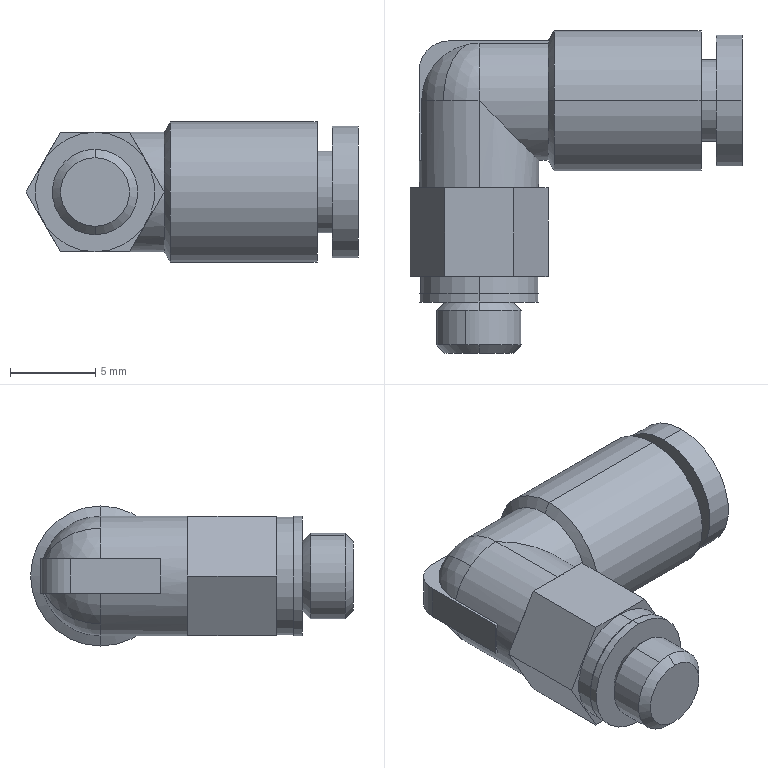Part | SolidWorks | features BaseBody 1 | 1 solid | 54 faces | box 19.441 x 18.9 x 8.2 mm | volume 1067 mm3 | plane 26 | cylinder 18 | cone 6 | sphere 4 | commonest cylinder face diameters 7 x5 4 x2 4.8 x2 5 x2 6.9 x2 7.7 x2
STEP:
#1=CARTESIAN_POINT('',(-3.354,11.8,-1.));
#2=VERTEX_POINT('',#1);
#3=CARTESIAN_POINT('',(-0.7454,15.07,-1.));
#4=VERTEX_POINT('',#3);
#5=CARTESIAN_POINT('',(0.,11.8,-1.));
#6=DIRECTION('',(0.,0.,-1.));
#7=DIRECTION('',(1.,0.,0.));
#8=AXIS2_PLACEMENT_3D('',#5,#6,#7);
#9=CIRCLE('',#8,3.354);
#10=EDGE_CURVE('',#2,#4,#9,.T.);
#11=ORIENTED_EDGE('',*,*,#10,.T.);
#12=CARTESIAN_POINT('',(-2.092,11.8,-2.806));
#13=VERTEX_POINT('',#12);
#14=CARTESIAN_POINT('',(0.,11.8,0.));
#15=DIRECTION('',(-0.8018,0.,0.5976));
#16=DIRECTION('',(0.5976,0.,0.8018));
#17=AXIS2_PLACEMENT_3D('',#14,#15,#16);
#18=CIRCLE('',#17,3.5);
#19=EDGE_CURVE('',#4,#13,#18,.T.);
#20=ORIENTED_EDGE('',*,*,#19,.T.);
#21=CARTESIAN_POINT('',(0.,11.8,0.));
#22=DIRECTION('',(0.,-1.,0.));
#23=DIRECTION('',(0.,0.,-1.));
#24=AXIS2_PLACEMENT_3D('',#21,#22,#23);
#25=CIRCLE('',#24,3.5);
#26=EDGE_CURVE('',#2,#13,#25,.T.);
#27=ORIENTED_EDGE('',*,*,#26,.F.);
#28=EDGE_LOOP('',(#11,#20,#27));
#29=FACE_OUTER_BOUND('',#28,.T.);
#30=CARTESIAN_POINT('',(0.,11.8,0.));
#31=DIRECTION('',(-0.8018,0.,0.5976));
#32=DIRECTION('',(0.5976,0.,0.8018));
#33=AXIS2_PLACEMENT_3D('',#30,#31,#32);
#34=SPHERICAL_SURFACE('',#33,3.5);
#35=ADVANCED_FACE('',(#29),#34,.T.);
#36=CARTESIAN_POINT('',(-0.7454,15.07,1.));
#37=VERTEX_POINT('',#36);
#38=CARTESIAN_POINT('',(0.,15.154,1.));
#39=VERTEX_POINT('',#38);
#40=CARTESIAN_POINT('',(0.,11.8,1.));
#41=DIRECTION('',(0.,0.,-1.));
#42=DIRECTION('',(1.,0.,0.));
#43=AXIS2_PLACEMENT_3D('',#40,#41,#42);
#44=CIRCLE('',#43,3.354);
#45=EDGE_CURVE('',#37,#39,#44,.T.);
#46=ORIENTED_EDGE('',*,*,#45,.F.);
#47=CARTESIAN_POINT('',(-2.092,11.8,2.806));
#48=VERTEX_POINT('',#47);
#49=CARTESIAN_POINT('',(0.,11.8,0.));
#50=DIRECTION('',(0.8018,0.,0.5976));
#51=DIRECTION('',(0.5976,0.,-0.8018));
#52=AXIS2_PLACEMENT_3D('',#49,#50,#51);
#53=CIRCLE('',#52,3.5);
#54=EDGE_CURVE('',#37,#48,#53,.T.);
#55=ORIENTED_EDGE('',*,*,#54,.T.);
#56=CARTESIAN_POINT('',(0.,11.8,3.5));
#57=VERTEX_POINT('',#56);
#58=CARTESIAN_POINT('',(0.,11.8,0.));
#59=DIRECTION('',(0.,-1.,0.));
#60=DIRECTION('',(0.,0.,-1.));
#61=AXIS2_PLACEMENT_3D('',#58,#59,#60);
#62=CIRCLE('',#61,3.5);
#63=EDGE_CURVE('',#57,#48,#62,.T.);
#64=ORIENTED_EDGE('',*,*,#63,.F.);
#65=CARTESIAN_POINT('',(0.,11.8,0.));
#66=DIRECTION('',(1.,0.,0.));
#67=DIRECTION('',(0.,0.,-1.));
#68=AXIS2_PLACEMENT_3D('',#65,#66,#67);
#69=CIRCLE('',#68,3.5);
#70=EDGE_CURVE('',#39,#57,#69,.T.);
#71=ORIENTED_EDGE('',*,*,#70,.F.);
#72=EDGE_LOOP('',(#46,#55,#64,#71));
#73=FACE_OUTER_BOUND('',#72,.T.);
#74=CARTESIAN_POINT('',(0.,11.8,0.));
#75=DIRECTION('',(0.8018,0.,0.5976));
#76=DIRECTION('',(0.5976,0.,-0.8018));
#77=AXIS2_PLACEMENT_3D('',#74,#75,#76);
#78=SPHERICAL_SURFACE('',#77,3.5);
#79=ADVANCED_FACE('',(#73),#78,.T.);
#80=CARTESIAN_POINT('',(0.,6.7,3.5));
#81=VERTEX_POINT('',#80);
#82=CARTESIAN_POINT('',(0.,11.8,3.5));
#83=DIRECTION('',(0.,-1.,0.));
#84=VECTOR('',#83,1000.);
#85=LINE('',#82,#84);
#86=EDGE_CURVE('',#57,#81,#85,.T.);
#87=ORIENTED_EDGE('',*,*,#86,.F.);
#88=ORIENTED_EDGE('',*,*,#63,.T.);
#89=CARTESIAN_POINT('',(-3.354,11.8,1.));
#90=VERTEX_POINT('',#89);
#91=CARTESIAN_POINT('',(0.,11.8,0.));
#92=DIRECTION('',(0.,-1.,0.));
#93=DIRECTION('',(0.,0.,-1.));
#94=AXIS2_PLACEMENT_3D('',#91,#92,#93);
#95=CIRCLE('',#94,3.5);
#96=EDGE_CURVE('',#48,#90,#95,.T.);
#97=ORIENTED_EDGE('',*,*,#96,.T.);
#98=CARTESIAN_POINT('',(-3.354,8.3,1.));
#99=VERTEX_POINT('',#98);
#100=CARTESIAN_POINT('',(-3.354,-3.,1.));
#101=DIRECTION('',(0.,-1.,0.));
#102=VECTOR('',#101,1000.);
#103=LINE('',#100,#102);
#104=EDGE_CURVE('',#90,#99,#103,.T.);
#105=ORIENTED_EDGE('',*,*,#104,.T.);
#106=CARTESIAN_POINT('',(-3.5,8.3,0.));
#107=VERTEX_POINT('',#106);
#108=CARTESIAN_POINT('',(0.,8.3,0.));
#109=DIRECTION('',(0.,1.,0.));
#110=DIRECTION('',(0.,0.,1.));
#111=AXIS2_PLACEMENT_3D('',#108,#109,#110);
#112=CIRCLE('',#111,3.5);
#113=EDGE_CURVE('',#107,#99,#112,.T.);
#114=ORIENTED_EDGE('',*,*,#113,.F.);
#115=CARTESIAN_POINT('',(-3.354,8.3,-1.));
#116=VERTEX_POINT('',#115);
#117=CARTESIAN_POINT('',(0.,8.3,0.));
#118=DIRECTION('',(0.,1.,0.));
#119=DIRECTION('',(0.,0.,1.));
#120=AXIS2_PLACEMENT_3D('',#117,#118,#119);
#121=CIRCLE('',#120,3.5);
#122=EDGE_CURVE('',#116,#107,#121,.T.);
#123=ORIENTED_EDGE('',*,*,#122,.F.);
#124=CARTESIAN_POINT('',(-3.354,-3.,-1.));
#125=DIRECTION('',(0.,-1.,0.));
#126=VECTOR('',#125,1000.);
#127=LINE('',#124,#126);
#128=EDGE_CURVE('',#2,#116,#127,.T.);
#129=ORIENTED_EDGE('',*,*,#128,.F.);
#130=ORIENTED_EDGE('',*,*,#26,.T.);
#131=CARTESIAN_POINT('',(0.,11.8,-3.5));
#132=VERTEX_POINT('',#131);
#133=CARTESIAN_POINT('',(0.,11.8,0.));
#134=DIRECTION('',(0.,-1.,0.));
#135=DIRECTION('',(0.,0.,-1.));
#136=AXIS2_PLACEMENT_3D('',#133,#134,#135);
#137=CIRCLE('',#136,3.5);
#138=EDGE_CURVE('',#13,#132,#137,.T.);
#139=ORIENTED_EDGE('',*,*,#138,.T.);
#140=CARTESIAN_POINT('',(0.,6.7,-3.5));
#141=VERTEX_POINT('',#140);
#142=CARTESIAN_POINT('',(0.,11.8,-3.5));
#143=DIRECTION('',(0.,-1.,0.));
#144=VECTOR('',#143,1000.);
#145=LINE('',#142,#144);
#146=EDGE_CURVE('',#132,#141,#145,.T.);
#147=ORIENTED_EDGE('',*,*,#146,.T.);
#148=CARTESIAN_POINT('',(-3.031,6.7,-1.75));
#149=VERTEX_POINT('',#148);
#150=CARTESIAN_POINT('',(0.,6.7,0.));
#151=DIRECTION('',(0.,-1.,0.));
#152=DIRECTION('',(0.,0.,-1.));
#153=AXIS2_PLACEMENT_3D('',#150,#151,#152);
#154=CIRCLE('',#153,3.5);
#155=EDGE_CURVE('',#149,#141,#154,.T.);
#156=ORIENTED_EDGE('',*,*,#155,.F.);
#157=CARTESIAN_POINT('',(-3.031,6.7,1.75));
#158=VERTEX_POINT('',#157);
#159=CARTESIAN_POINT('',(0.,6.7,0.));
#160=DIRECTION('',(0.,-1.,0.));
#161=DIRECTION('',(0.,0.,-1.));
#162=AXIS2_PLACEMENT_3D('',#159,#160,#161);
#163=CIRCLE('',#162,3.5);
#164=EDGE_CURVE('',#158,#149,#163,.T.);
#165=ORIENTED_EDGE('',*,*,#164,.F.);
#166=CARTESIAN_POINT('',(0.,6.7,0.));
#167=DIRECTION('',(0.,-1.,0.));
#168=DIRECTION('',(0.,0.,-1.));
#169=AXIS2_PLACEMENT_3D('',#166,#167,#168);
#170=CIRCLE('',#169,3.5);
#171=EDGE_CURVE('',#81,#158,#170,.T.);
#172=ORIENTED_EDGE('',*,*,#171,.F.);
#173=EDGE_LOOP('',(#87,#88,#97,#105,#114,#123,#129,#130,#139,#147,#156,#165,#172));
#174=FACE_OUTER_BOUND('',#173,.T.);
#175=CARTESIAN_POINT('',(0.,-3.,0.));
#176=DIRECTION('',(0.,-1.,0.));
#177=DIRECTION('',(1.,0.,0.));
#178=AXIS2_PLACEMENT_3D('',#175,#176,#177);
#179=CYLINDRICAL_SURFACE('',#178,3.5);
#180=ADVANCED_FACE('',(#174),#179,.T.);
#181=CARTESIAN_POINT('',(-2.021,6.7,3.5));
#182=VERTEX_POINT('',#181);
#183=CARTESIAN_POINT('',(-2.156,6.7,3.266));
#184=DIRECTION('',(0.5,0.,0.866));
#185=VECTOR('',#184,1000.);
#186=LINE('',#183,#185);
#187=EDGE_CURVE('',#158,#182,#186,.T.);
#188=ORIENTED_EDGE('',*,*,#187,.T.);
#189=CARTESIAN_POINT('',(3.5,6.7,3.5));
#190=DIRECTION('',(1.,0.,0.));
#191=VECTOR('',#190,1000.);
#192=LINE('',#189,#191);
#193=EDGE_CURVE('',#182,#81,#192,.T.);
#194=ORIENTED_EDGE('',*,*,#193,.T.);
#195=ORIENTED_EDGE('',*,*,#171,.T.);
#196=EDGE_LOOP('',(#188,#194,#195));
#197=FACE_OUTER_BOUND('',#196,.T.);
#198=CARTESIAN_POINT('',(3.5,6.7,0.));
#199=DIRECTION('',(0.,-1.,0.));
#200=DIRECTION('',(0.,0.,-1.));
#201=AXIS2_PLACEMENT_3D('',#198,#199,#200);
#202=PLANE('',#201);
#203=ADVANCED_FACE('',(#197),#202,.F.);
#204=CARTESIAN_POINT('',(-2.021,1.5,3.5));
#205=VERTEX_POINT('',#204);
#206=CARTESIAN_POINT('',(-2.021,8.3,3.5));
#207=DIRECTION('',(0.,-1.,0.));
#208=VECTOR('',#207,1000.);
#209=LINE('',#206,#208);
#210=EDGE_CURVE('',#182,#205,#209,.T.);
#211=ORIENTED_EDGE('',*,*,#210,.T.);
#212=CARTESIAN_POINT('',(2.021,1.5,3.5));
#213=VERTEX_POINT('',#212);
#214=CARTESIAN_POINT('',(4.2,1.5,3.5));
#215=DIRECTION('',(-1.,0.,0.));
#216=VECTOR('',#215,1000.);
#217=LINE('',#214,#216);
#218=EDGE_CURVE('',#213,#205,#217,.T.);
#219=ORIENTED_EDGE('',*,*,#218,.F.);
#220=CARTESIAN_POINT('',(2.021,6.7,3.5));
#221=VERTEX_POINT('',#220);
#222=CARTESIAN_POINT('',(2.021,8.3,3.5));
#223=DIRECTION('',(0.,-1.,0.));
#224=VECTOR('',#223,1000.);
#225=LINE('',#222,#224);
#226=EDGE_CURVE('',#221,#213,#225,.T.);
#227=ORIENTED_EDGE('',*,*,#226,.F.);
#228=CARTESIAN_POINT('',(3.5,6.7,3.5));
#229=DIRECTION('',(1.,0.,0.));
#230=VECTOR('',#229,1000.);
#231=LINE('',#228,#230);
#232=EDGE_CURVE('',#81,#221,#231,.T.);
#233=ORIENTED_EDGE('',*,*,#232,.F.);
#234=ORIENTED_EDGE('',*,*,#193,.F.);
#235=EDGE_LOOP('',(#211,#219,#227,#233,#234));
#236=FACE_OUTER_BOUND('',#235,.T.);
#237=CARTESIAN_POINT('',(-2.021,8.3,3.5));
#238=DIRECTION('',(0.,0.,-1.));
#239=DIRECTION('',(-1.,0.,0.));
#240=AXIS2_PLACEMENT_3D('',#237,#238,#239);
#241=PLANE('',#240);
#242=ADVANCED_FACE('',(#236),#241,.F.);
#243=ORIENTED_EDGE('',*,*,#232,.T.);
#244=CARTESIAN_POINT('',(3.031,6.7,1.75));
#245=VERTEX_POINT('',#244);
#246=CARTESIAN_POINT('',(3.906,6.7,0.2345));
#247=DIRECTION('',(0.5,0.,-0.866));
#248=VECTOR('',#247,1000.);
#249=LINE('',#246,#248);
#250=EDGE_CURVE('',#221,#245,#249,.T.);
#251=ORIENTED_EDGE('',*,*,#250,.T.);
#252=CARTESIAN_POINT('',(0.,6.7,0.));
#253=DIRECTION('',(0.,-1.,0.));
#254=DIRECTION('',(0.,0.,-1.));
#255=AXIS2_PLACEMENT_3D('',#252,#253,#254);
#256=CIRCLE('',#255,3.5);
#257=EDGE_CURVE('',#245,#81,#256,.T.);
#258=ORIENTED_EDGE('',*,*,#257,.T.);
#259=EDGE_LOOP('',(#243,#251,#258));
#260=FACE_OUTER_BOUND('',#259,.T.);
#261=CARTESIAN_POINT('',(3.5,6.7,0.));
#262=DIRECTION('',(0.,-1.,0.));
#263=DIRECTION('',(0.,0.,-1.));
#264=AXIS2_PLACEMENT_3D('',#261,#262,#263);
#265=PLANE('',#264);
#266=ADVANCED_FACE('',(#260),#265,.F.);
#267=ORIENTED_EDGE('',*,*,#86,.T.);
#268=ORIENTED_EDGE('',*,*,#257,.F.);
#269=CARTESIAN_POINT('',(3.031,6.7,-1.75));
#270=VERTEX_POINT('',#269);
#271=CARTESIAN_POINT('',(0.,6.7,0.));
#272=DIRECTION('',(0.,-1.,0.));
#273=DIRECTION('',(0.,0.,-1.));
#274=AXIS2_PLACEMENT_3D('',#271,#272,#273);
#275=CIRCLE('',#274,3.5);
#276=EDGE_CURVE('',#270,#245,#275,.T.);
#277=ORIENTED_EDGE('',*,*,#276,.F.);
#278=CARTESIAN_POINT('',(0.,6.7,0.));
#279=DIRECTION('',(0.,-1.,0.));
#280=DIRECTION('',(0.,0.,-1.));
#281=AXIS2_PLACEMENT_3D('',#278,#279,#280);
#282=CIRCLE('',#281,3.5);
#283=EDGE_CURVE('',#141,#270,#282,.T.);
#284=ORIENTED_EDGE('',*,*,#283,.F.);
#285=ORIENTED_EDGE('',*,*,#146,.F.);
#286=CARTESIAN_POINT('',(0.,11.8,3.5));
#287=CARTESIAN_POINT('',(0.4581,11.342,3.5));
#288=CARTESIAN_POINT('',(0.9161,10.884,3.409));
#289=CARTESIAN_POINT('',(1.763,10.037,3.058));
#290=CARTESIAN_POINT('',(2.151,9.649,2.799));
#291=CARTESIAN_POINT('',(2.799,9.001,2.151));
#292=CARTESIAN_POINT('',(3.058,8.742,1.763));
#293=CARTESIAN_POINT('',(3.409,8.391,0.9161));
#294=CARTESIAN_POINT('',(3.5,8.3,0.4581));
#295=CARTESIAN_POINT('',(3.5,8.3,-0.4581));
#296=CARTESIAN_POINT('',(3.409,8.391,-0.9161));
#297=CARTESIAN_POINT('',(3.058,8.742,-1.763));
#298=CARTESIAN_POINT('',(2.799,9.001,-2.151));
#299=CARTESIAN_POINT('',(2.151,9.649,-2.799));
#300=CARTESIAN_POINT('',(1.763,10.037,-3.058));
#301=CARTESIAN_POINT('',(0.9161,10.884,-3.409));
#302=CARTESIAN_POINT('',(0.4581,11.342,-3.5));
#303=CARTESIAN_POINT('',(0.,11.8,-3.5));
#304=B_SPLINE_CURVE_WITH_KNOTS('',3,(#286,#287,#288,#289,#290,#291,#292,#293,#294,#295,#296,#297,#298,#299,#300,#301,#302,#303),.UNSPECIFIED.,.F.,.F.,(4,2,2,2,2,2,2,2,4),(0.,0.125,0.25,0.375,0.5,0.625,0.75,0.875,1.),.UNSPECIFIED.);
#305=EDGE_CURVE('',#57,#132,#304,.T.);
#306=ORIENTED_EDGE('',*,*,#305,.F.);
#307=EDGE_LOOP('',(#267,#268,#277,#284,#285,#306));
#308=FACE_OUTER_BOUND('',#307,.T.);
#309=CARTESIAN_POINT('',(0.,-3.,0.));
#310=DIRECTION('',(0.,-1.,0.));
#311=DIRECTION('',(-1.,0.,0.));
#312=AXIS2_PLACEMENT_3D('',#309,#310,#311);
#313=CYLINDRICAL_SURFACE('',#312,3.5);
#314=ADVANCED_FACE('',(#308),#313,.T.);
#315=CARTESIAN_POINT('',(4.054,11.8,-3.5));
#316=VERTEX_POINT('',#315);
#317=CARTESIAN_POINT('',(4.054,15.154,-1.));
#318=VERTEX_POINT('',#317);
#319=CARTESIAN_POINT('',(4.054,11.8,0.));
#320=DIRECTION('',(1.,0.,0.));
#321=DIRECTION('',(0.,0.,-1.));
#322=AXIS2_PLACEMENT_3D('',#319,#320,#321);
#323=CIRCLE('',#322,3.5);
#324=EDGE_CURVE('',#316,#318,#323,.T.);
#325=ORIENTED_EDGE('',*,*,#324,.F.);
#326=CARTESIAN_POINT('',(4.054,11.8,3.5));
#327=VERTEX_POINT('',#326);
#328=CARTESIAN_POINT('',(4.054,11.8,0.));
#329=DIRECTION('',(1.,0.,0.));
#330=DIRECTION('',(0.,0.,-1.));
#331=AXIS2_PLACEMENT_3D('',#328,#329,#330);
#332=CIRCLE('',#331,3.5);
#333=EDGE_CURVE('',#327,#316,#332,.T.);
#334=ORIENTED_EDGE('',*,*,#333,.F.);
#335=CARTESIAN_POINT('',(4.054,15.154,1.));
#336=VERTEX_POINT('',#335);
#337=CARTESIAN_POINT('',(4.054,11.8,0.));
#338=DIRECTION('',(1.,0.,0.));
#339=DIRECTION('',(0.,0.,-1.));
#340=AXIS2_PLACEMENT_3D('',#337,#338,#339);
#341=CIRCLE('',#340,3.5);
#342=EDGE_CURVE('',#336,#327,#341,.T.);
#343=ORIENTED_EDGE('',*,*,#342,.F.);
#344=CARTESIAN_POINT('',(15.4,15.154,1.));
#345=DIRECTION('',(-1.,0.,0.));
#346=VECTOR('',#345,1000.);
#347=LINE('',#344,#346);
#348=EDGE_CURVE('',#336,#39,#347,.T.);
#349=ORIENTED_EDGE('',*,*,#348,.T.);
#350=ORIENTED_EDGE('',*,*,#70,.T.);
#351=ORIENTED_EDGE('',*,*,#305,.T.);
#352=CARTESIAN_POINT('',(0.,15.154,-1.));
#353=VERTEX_POINT('',#352);
#354=CARTESIAN_POINT('',(0.,11.8,0.));
#355=DIRECTION('',(1.,0.,0.));
#356=DIRECTION('',(0.,0.,-1.));
#357=AXIS2_PLACEMENT_3D('',#354,#355,#356);
#358=CIRCLE('',#357,3.5);
#359=EDGE_CURVE('',#132,#353,#358,.T.);
#360=ORIENTED_EDGE('',*,*,#359,.T.);
#361=CARTESIAN_POINT('',(15.4,15.154,-1.));
#362=DIRECTION('',(-1.,0.,0.));
#363=VECTOR('',#362,1000.);
#364=LINE('',#361,#363);
#365=EDGE_CURVE('',#318,#353,#364,.T.);
#366=ORIENTED_EDGE('',*,*,#365,.F.);
#367=EDGE_LOOP('',(#325,#334,#343,#349,#350,#351,#360,#366));
#368=FACE_OUTER_BOUND('',#367,.T.);
#369=CARTESIAN_POINT('',(15.4,11.8,0.));
#370=DIRECTION('',(1.,0.,0.));
#371=DIRECTION('',(0.,1.,0.));
#372=AXIS2_PLACEMENT_3D('',#369,#370,#371);
#373=CYLINDRICAL_SURFACE('',#372,3.5);
#374=ADVANCED_FACE('',(#368),#373,.T.);
#375=ORIENTED_EDGE('',*,*,#10,.F.);
#376=ORIENTED_EDGE('',*,*,#128,.T.);
#377=CARTESIAN_POINT('',(-3.5,8.3,-1.));
#378=VERTEX_POINT('',#377);
#379=CARTESIAN_POINT('',(-3.5,8.3,-1.));
#380=DIRECTION('',(1.,0.,0.));
#381=VECTOR('',#380,1000.);
#382=LINE('',#379,#381);
#383=EDGE_CURVE('',#378,#116,#382,.T.);
#384=ORIENTED_EDGE('',*,*,#383,.F.);
#385=CARTESIAN_POINT('',(-3.5,13.55,-1.));
#386=VERTEX_POINT('',#385);
#387=CARTESIAN_POINT('',(-3.5,13.55,-1.));
#388=DIRECTION('',(0.,-1.,0.));
#389=VECTOR('',#388,1000.);
#390=LINE('',#387,#389);
#391=EDGE_CURVE('',#386,#378,#390,.T.);
#392=ORIENTED_EDGE('',*,*,#391,.F.);
#393=CARTESIAN_POINT('',(-1.75,15.3,-1.));
#394=VERTEX_POINT('',#393);
#395=CARTESIAN_POINT('',(-1.75,13.55,-1.));
#396=DIRECTION('',(0.,0.,1.));
#397=DIRECTION('',(1.,0.,0.));
#398=AXIS2_PLACEMENT_3D('',#395,#396,#397);
#399=CIRCLE('',#398,1.75);
#400=EDGE_CURVE('',#394,#386,#399,.T.);
#401=ORIENTED_EDGE('',*,*,#400,.F.);
#402=CARTESIAN_POINT('',(4.134,15.3,-1.));
#403=VERTEX_POINT('',#402);
#404=CARTESIAN_POINT('',(4.4,15.3,-1.));
#405=DIRECTION('',(-1.,0.,0.));
#406=VECTOR('',#405,1000.);
#407=LINE('',#404,#406);
#408=EDGE_CURVE('',#403,#394,#407,.T.);
#409=ORIENTED_EDGE('',*,*,#408,.F.);
#410=CARTESIAN_POINT('',(4.134,15.3,-1.));
#411=CARTESIAN_POINT('',(4.108,15.252,-1.));
#412=CARTESIAN_POINT('',(4.081,15.203,-1.));
#413=CARTESIAN_POINT('',(4.054,15.154,-1.));
#414=B_SPLINE_CURVE_WITH_KNOTS('',3,(#410,#411,#412,#413),.UNSPECIFIED.,.F.,.F.,(4,4),(0.,1.),.UNSPECIFIED.);
#415=EDGE_CURVE('',#403,#318,#414,.T.);
#416=ORIENTED_EDGE('',*,*,#415,.T.);
#417=ORIENTED_EDGE('',*,*,#365,.T.);
#418=CARTESIAN_POINT('',(0.,11.8,-1.));
#419=DIRECTION('',(0.,0.,-1.));
#420=DIRECTION('',(1.,0.,0.));
#421=AXIS2_PLACEMENT_3D('',#418,#419,#420);
#422=CIRCLE('',#421,3.354);
#423=EDGE_CURVE('',#4,#353,#422,.T.);
#424=ORIENTED_EDGE('',*,*,#423,.F.);
#425=EDGE_LOOP('',(#375,#376,#384,#392,#401,#409,#416,#417,#424));
#426=FACE_OUTER_BOUND('',#425,.T.);
#427=CARTESIAN_POINT('',(-1.75,13.55,-1.));
#428=DIRECTION('',(0.,0.,1.));
#429=DIRECTION('',(1.,0.,0.));
#430=AXIS2_PLACEMENT_3D('',#427,#428,#429);
#431=PLANE('',#430);
#432=ADVANCED_FACE('',(#426),#431,.F.);
#433=CARTESIAN_POINT('',(4.4,11.8,4.1));
#434=VERTEX_POINT('',#433);
#435=CARTESIAN_POINT('',(4.054,11.8,3.5));
#436=DIRECTION('',(0.5,0.,0.866));
#437=VECTOR('',#436,1000.);
#438=LINE('',#435,#437);
#439=EDGE_CURVE('',#327,#434,#438,.T.);
#440=ORIENTED_EDGE('',*,*,#439,.T.);
#441=CARTESIAN_POINT('',(4.4,11.8,-4.1));
#442=VERTEX_POINT('',#441);
#443=CARTESIAN_POINT('',(4.4,11.8,0.));
#444=DIRECTION('',(1.,0.,0.));
#445=DIRECTION('',(0.,0.,-1.));
#446=AXIS2_PLACEMENT_3D('',#443,#444,#445);
#447=CIRCLE('',#446,4.1);
#448=EDGE_CURVE('',#442,#434,#447,.T.);
#449=ORIENTED_EDGE('',*,*,#448,.F.);
#450=CARTESIAN_POINT('',(4.054,11.8,-3.5));
#451=DIRECTION('',(0.5,0.,-0.866));
#452=VECTOR('',#451,1000.);
#453=LINE('',#450,#452);
#454=EDGE_CURVE('',#316,#442,#453,.T.);
#455=ORIENTED_EDGE('',*,*,#454,.F.);
#456=ORIENTED_EDGE('',*,*,#324,.T.);
#457=ORIENTED_EDGE('',*,*,#415,.F.);
#458=CARTESIAN_POINT('',(4.134,15.3,1.));
#459=VERTEX_POINT('',#458);
#460=CARTESIAN_POINT('',(4.134,15.3,1.));
#461=CARTESIAN_POINT('',(4.083,15.3,0.6726));
#462=CARTESIAN_POINT('',(4.054,15.3,0.3321));
#463=CARTESIAN_POINT('',(4.054,15.3,-0.1679));
#464=CARTESIAN_POINT('',(4.061,15.3,-0.3341));
#465=CARTESIAN_POINT('',(4.088,15.3,-0.669));
#466=CARTESIAN_POINT('',(4.108,15.3,-0.8363));
#467=CARTESIAN_POINT('',(4.134,15.3,-1.));
#468=B_SPLINE_CURVE_WITH_KNOTS('',3,(#460,#461,#462,#463,#464,#465,#466,#467),.UNSPECIFIED.,.F.,.F.,(4,2,2,4),(0.,0.5,0.75,1.),.UNSPECIFIED.);
#469=EDGE_CURVE('',#459,#403,#468,.T.);
#470=ORIENTED_EDGE('',*,*,#469,.F.);
#471=CARTESIAN_POINT('',(4.134,15.3,1.));
#472=CARTESIAN_POINT('',(4.108,15.252,1.));
#473=CARTESIAN_POINT('',(4.081,15.203,1.));
#474=CARTESIAN_POINT('',(4.054,15.154,1.));
#475=B_SPLINE_CURVE_WITH_KNOTS('',3,(#471,#472,#473,#474),.UNSPECIFIED.,.F.,.F.,(4,4),(0.,1.),.UNSPECIFIED.);
#476=EDGE_CURVE('',#459,#336,#475,.T.);
#477=ORIENTED_EDGE('',*,*,#476,.T.);
#478=ORIENTED_EDGE('',*,*,#342,.T.);
#479=EDGE_LOOP('',(#440,#449,#455,#456,#457,#470,#477,#478));
#480=FACE_OUTER_BOUND('',#479,.T.);
#481=CARTESIAN_POINT('',(4.054,11.8,0.));
#482=DIRECTION('',(1.,0.,0.));
#483=DIRECTION('',(0.,-1.,0.));
#484=AXIS2_PLACEMENT_3D('',#481,#482,#483);
#485=CONICAL_SURFACE('',#484,3.5,1.047);
#486=ADVANCED_FACE('',(#480),#485,.T.);
#487=ORIENTED_EDGE('',*,*,#104,.F.);
#488=CARTESIAN_POINT('',(0.,11.8,1.));
#489=DIRECTION('',(0.,0.,-1.));
#490=DIRECTION('',(1.,0.,0.));
#491=AXIS2_PLACEMENT_3D('',#488,#489,#490);
#492=CIRCLE('',#491,3.354);
#493=EDGE_CURVE('',#90,#37,#492,.T.);
#494=ORIENTED_EDGE('',*,*,#493,.T.);
#495=ORIENTED_EDGE('',*,*,#45,.T.);
#496=ORIENTED_EDGE('',*,*,#348,.F.);
#497=ORIENTED_EDGE('',*,*,#476,.F.);
#498=CARTESIAN_POINT('',(-1.75,15.3,1.));
#499=VERTEX_POINT('',#498);
#500=CARTESIAN_POINT('',(4.4,15.3,1.));
#501=DIRECTION('',(-1.,0.,0.));
#502=VECTOR('',#501,1000.);
#503=LINE('',#500,#502);
#504=EDGE_CURVE('',#459,#499,#503,.T.);
#505=ORIENTED_EDGE('',*,*,#504,.T.);
#506=CARTESIAN_POINT('',(-3.5,13.55,1.));
#507=VERTEX_POINT('',#506);
#508=CARTESIAN_POINT('',(-1.75,13.55,1.));
#509=DIRECTION('',(0.,0.,1.));
#510=DIRECTION('',(1.,0.,0.));
#511=AXIS2_PLACEMENT_3D('',#508,#509,#510);
#512=CIRCLE('',#511,1.75);
#513=EDGE_CURVE('',#499,#507,#512,.T.);
#514=ORIENTED_EDGE('',*,*,#513,.T.);
#515=CARTESIAN_POINT('',(-3.5,8.3,1.));
#516=VERTEX_POINT('',#515);
#517=CARTESIAN_POINT('',(-3.5,13.55,1.));
#518=DIRECTION('',(0.,-1.,0.));
#519=VECTOR('',#518,1000.);
#520=LINE('',#517,#519);
#521=EDGE_CURVE('',#507,#516,#520,.T.);
#522=ORIENTED_EDGE('',*,*,#521,.T.);
#523=CARTESIAN_POINT('',(-3.5,8.3,1.));
#524=DIRECTION('',(1.,0.,0.));
#525=VECTOR('',#524,1000.);
#526=LINE('',#523,#525);
#527=EDGE_CURVE('',#516,#99,#526,.T.);
#528=ORIENTED_EDGE('',*,*,#527,.T.);
#529=EDGE_LOOP('',(#487,#494,#495,#496,#497,#505,#514,#522,#528));
#530=FACE_OUTER_BOUND('',#529,.T.);
#531=CARTESIAN_POINT('',(-1.75,13.55,1.));
#532=DIRECTION('',(0.,0.,1.));
#533=DIRECTION('',(1.,0.,0.));
#534=AXIS2_PLACEMENT_3D('',#531,#532,#533);
#535=PLANE('',#534);
#536=ADVANCED_FACE('',(#530),#535,.T.);
#537=CARTESIAN_POINT('',(-3.5,8.3,1.));
#538=DIRECTION('',(0.,0.,-1.));
#539=VECTOR('',#538,1000.);
#540=LINE('',#537,#539);
#541=EDGE_CURVE('',#516,#107,#540,.T.);
#542=ORIENTED_EDGE('',*,*,#541,.T.);
#543=ORIENTED_EDGE('',*,*,#113,.T.);
#544=ORIENTED_EDGE('',*,*,#527,.F.);
#545=EDGE_LOOP('',(#542,#543,#544));
#546=FACE_OUTER_BOUND('',#545,.T.);
#547=CARTESIAN_POINT('',(-3.5,8.3,1.));
#548=DIRECTION('',(0.,1.,0.));
#549=DIRECTION('',(0.,0.,1.));
#550=AXIS2_PLACEMENT_3D('',#547,#548,#549);
#551=PLANE('',#550);
#552=ADVANCED_FACE('',(#546),#551,.F.);
#553=CARTESIAN_POINT('',(-3.5,8.3,1.));
#554=DIRECTION('',(0.,0.,-1.));
#555=VECTOR('',#554,1000.);
#556=LINE('',#553,#555);
#557=EDGE_CURVE('',#107,#378,#556,.T.);
#558=ORIENTED_EDGE('',*,*,#557,.F.);
#559=ORIENTED_EDGE('',*,*,#541,.F.);
#560=ORIENTED_EDGE('',*,*,#521,.F.);
#561=CARTESIAN_POINT('',(-3.5,13.55,1.));
#562=DIRECTION('',(0.,0.,-1.));
#563=VECTOR('',#562,1000.);
#564=LINE('',#561,#563);
#565=EDGE_CURVE('',#507,#386,#564,.T.);
#566=ORIENTED_EDGE('',*,*,#565,.T.);
#567=ORIENTED_EDGE('',*,*,#391,.T.);
#568=EDGE_LOOP('',(#558,#559,#560,#566,#567));
#569=FACE_OUTER_BOUND('',#568,.T.);
#570=CARTESIAN_POINT('',(-3.5,13.55,1.));
#571=DIRECTION('',(1.,0.,0.));
#572=DIRECTION('',(0.,0.,-1.));
#573=AXIS2_PLACEMENT_3D('',#570,#571,#572);
#574=PLANE('',#573);
#575=ADVANCED_FACE('',(#569),#574,.F.);
#576=ORIENTED_EDGE('',*,*,#400,.T.);
#577=ORIENTED_EDGE('',*,*,#565,.F.);
#578=ORIENTED_EDGE('',*,*,#513,.F.);
#579=CARTESIAN_POINT('',(-1.75,15.3,1.));
#580=DIRECTION('',(0.,0.,-1.));
#581=VECTOR('',#580,1000.);
#582=LINE('',#579,#581);
#583=EDGE_CURVE('',#499,#394,#582,.T.);
#584=ORIENTED_EDGE('',*,*,#583,.T.);
#585=EDGE_LOOP('',(#576,#577,#578,#584));
#586=FACE_OUTER_BOUND('',#585,.T.);
#587=CARTESIAN_POINT('',(-1.75,13.55,1.));
#588=DIRECTION('',(0.,0.,-1.));
#589=DIRECTION('',(0.7071,-0.7071,0.));
#590=AXIS2_PLACEMENT_3D('',#587,#588,#589);
#591=CYLINDRICAL_SURFACE('',#590,1.75);
#592=ADVANCED_FACE('',(#586),#591,.T.);
#593=ORIENTED_EDGE('',*,*,#504,.F.);
#594=ORIENTED_EDGE('',*,*,#469,.T.);
#595=ORIENTED_EDGE('',*,*,#408,.T.);
#596=ORIENTED_EDGE('',*,*,#583,.F.);
#597=EDGE_LOOP('',(#593,#594,#595,#596));
#598=FACE_OUTER_BOUND('',#597,.T.);
#599=CARTESIAN_POINT('',(4.4,15.3,1.));
#600=DIRECTION('',(0.,-1.,0.));
#601=DIRECTION('',(0.,0.,-1.));
#602=AXIS2_PLACEMENT_3D('',#599,#600,#601);
#603=PLANE('',#602);
#604=ADVANCED_FACE('',(#598),#603,.F.);
#605=ORIENTED_EDGE('',*,*,#383,.T.);
#606=ORIENTED_EDGE('',*,*,#122,.T.);
#607=ORIENTED_EDGE('',*,*,#557,.T.);
#608=EDGE_LOOP('',(#605,#606,#607));
#609=FACE_OUTER_BOUND('',#608,.T.);
#610=CARTESIAN_POINT('',(-3.5,8.3,1.));
#611=DIRECTION('',(0.,1.,0.));
#612=DIRECTION('',(0.,0.,1.));
#613=AXIS2_PLACEMENT_3D('',#610,#611,#612);
#614=PLANE('',#613);
#615=ADVANCED_FACE('',(#609),#614,.F.);
#616=ORIENTED_EDGE('',*,*,#54,.F.);
#617=ORIENTED_EDGE('',*,*,#493,.F.);
#618=ORIENTED_EDGE('',*,*,#96,.F.);
#619=EDGE_LOOP('',(#616,#617,#618));
#620=FACE_OUTER_BOUND('',#619,.T.);
#621=CARTESIAN_POINT('',(0.,11.8,0.));
#622=DIRECTION('',(0.8018,0.,0.5976));
#623=DIRECTION('',(0.5976,0.,-0.8018));
#624=AXIS2_PLACEMENT_3D('',#621,#622,#623);
#625=SPHERICAL_SURFACE('',#624,3.5);
#626=ADVANCED_FACE('',(#620),#625,.T.);
#627=ORIENTED_EDGE('',*,*,#439,.F.);
#628=ORIENTED_EDGE('',*,*,#333,.T.);
#629=ORIENTED_EDGE('',*,*,#454,.T.);
#630=CARTESIAN_POINT('',(4.4,11.8,0.));
#631=DIRECTION('',(1.,0.,0.));
#632=DIRECTION('',(0.,0.,-1.));
#633=AXIS2_PLACEMENT_3D('',#630,#631,#632);
#634=CIRCLE('',#633,4.1);
#635=EDGE_CURVE('',#434,#442,#634,.T.);
#636=ORIENTED_EDGE('',*,*,#635,.F.);
#637=EDGE_LOOP('',(#627,#628,#629,#636));
#638=FACE_OUTER_BOUND('',#637,.T.);
#639=CARTESIAN_POINT('',(4.054,11.8,0.));
#640=DIRECTION('',(1.,0.,0.));
#641=DIRECTION('',(0.,1.,0.));
#642=AXIS2_PLACEMENT_3D('',#639,#640,#641);
#643=CONICAL_SURFACE('',#642,3.5,1.047);
#644=ADVANCED_FACE('',(#638),#643,.T.);
#645=CARTESIAN_POINT('',(13.,11.8,4.1));
#646=VERTEX_POINT('',#645);
#647=CARTESIAN_POINT('',(4.4,11.8,4.1));
#648=DIRECTION('',(1.,0.,0.));
#649=VECTOR('',#648,1000.);
#650=LINE('',#647,#649);
#651=EDGE_CURVE('',#434,#646,#650,.T.);
#652=ORIENTED_EDGE('',*,*,#651,.F.);
#653=ORIENTED_EDGE('',*,*,#635,.T.);
#654=CARTESIAN_POINT('',(13.,11.8,-4.1));
#655=VERTEX_POINT('',#654);
#656=CARTESIAN_POINT('',(4.4,11.8,-4.1));
#657=DIRECTION('',(1.,0.,0.));
#658=VECTOR('',#657,1000.);
#659=LINE('',#656,#658);
#660=EDGE_CURVE('',#442,#655,#659,.T.);
#661=ORIENTED_EDGE('',*,*,#660,.T.);
#662=CARTESIAN_POINT('',(13.,11.8,0.));
#663=DIRECTION('',(1.,0.,0.));
#664=DIRECTION('',(0.,0.,-1.));
#665=AXIS2_PLACEMENT_3D('',#662,#663,#664);
#666=CIRCLE('',#665,4.1);
#667=EDGE_CURVE('',#646,#655,#666,.T.);
#668=ORIENTED_EDGE('',*,*,#667,.F.);
#669=EDGE_LOOP('',(#652,#653,#661,#668));
#670=FACE_OUTER_BOUND('',#669,.T.);
#671=CARTESIAN_POINT('',(15.4,11.8,0.));
#672=DIRECTION('',(1.,0.,0.));
#673=DIRECTION('',(0.,1.,0.));
#674=AXIS2_PLACEMENT_3D('',#671,#672,#673);
#675=CYLINDRICAL_SURFACE('',#674,4.1);
#676=ADVANCED_FACE('',(#670),#675,.T.);
#677=CARTESIAN_POINT('',(13.,11.8,2.4));
#678=VERTEX_POINT('',#677);
#679=CARTESIAN_POINT('',(13.,11.8,-2.4));
#680=VERTEX_POINT('',#679);
#681=CARTESIAN_POINT('',(13.,11.8,0.));
#682=DIRECTION('',(1.,0.,0.));
#683=DIRECTION('',(0.,0.,-1.));
#684=AXIS2_PLACEMENT_3D('',#681,#682,#683);
#685=CIRCLE('',#684,2.4);
#686=EDGE_CURVE('',#678,#680,#685,.T.);
#687=ORIENTED_EDGE('',*,*,#686,.F.);
#688=CARTESIAN_POINT('',(13.,11.8,0.));
#689=DIRECTION('',(1.,0.,0.));
#690=DIRECTION('',(0.,0.,-1.));
#691=AXIS2_PLACEMENT_3D('',#688,#689,#690);
#692=CIRCLE('',#691,2.4);
#693=EDGE_CURVE('',#680,#678,#692,.T.);
#694=ORIENTED_EDGE('',*,*,#693,.F.);
#695=EDGE_LOOP('',(#687,#694));
#696=FACE_BOUND('',#695,.T.);
#697=CARTESIAN_POINT('',(13.,11.8,0.));
#698=DIRECTION('',(1.,0.,0.));
#699=DIRECTION('',(0.,0.,-1.));
#700=AXIS2_PLACEMENT_3D('',#697,#698,#699);
#701=CIRCLE('',#700,4.1);
#702=EDGE_CURVE('',#655,#646,#701,.T.);
#703=ORIENTED_EDGE('',*,*,#702,.T.);
#704=ORIENTED_EDGE('',*,*,#667,.T.);
#705=EDGE_LOOP('',(#703,#704));
#706=FACE_OUTER_BOUND('',#705,.T.);
#707=CARTESIAN_POINT('',(13.,15.9,0.));
#708=DIRECTION('',(-1.,0.,0.));
#709=DIRECTION('',(0.,0.,1.));
#710=AXIS2_PLACEMENT_3D('',#707,#708,#709);
#711=PLANE('',#710);
#712=ADVANCED_FACE('',(#696,#706),#711,.F.);
#713=ORIENTED_EDGE('',*,*,#651,.T.);
#714=ORIENTED_EDGE('',*,*,#702,.F.);
#715=ORIENTED_EDGE('',*,*,#660,.F.);
#716=ORIENTED_EDGE('',*,*,#448,.T.);
#717=EDGE_LOOP('',(#713,#714,#715,#716));
#718=FACE_OUTER_BOUND('',#717,.T.);
#719=CARTESIAN_POINT('',(15.4,11.8,0.));
#720=DIRECTION('',(1.,0.,0.));
#721=DIRECTION('',(0.,-1.,0.));
#722=AXIS2_PLACEMENT_3D('',#719,#720,#721);
#723=CYLINDRICAL_SURFACE('',#722,4.1);
#724=ADVANCED_FACE('',(#718),#723,.T.);
#725=CARTESIAN_POINT('',(13.9,11.8,2.4));
#726=VERTEX_POINT('',#725);
#727=CARTESIAN_POINT('',(13.,11.8,2.4));
#728=DIRECTION('',(1.,0.,0.));
#729=VECTOR('',#728,1000.);
#730=LINE('',#727,#729);
#731=EDGE_CURVE('',#678,#726,#730,.T.);
#732=ORIENTED_EDGE('',*,*,#731,.T.);
#733=CARTESIAN_POINT('',(13.9,11.8,-2.4));
#734=VERTEX_POINT('',#733);
#735=CARTESIAN_POINT('',(13.9,11.8,0.));
#736=DIRECTION('',(1.,0.,0.));
#737=DIRECTION('',(0.,0.,-1.));
#738=AXIS2_PLACEMENT_3D('',#735,#736,#737);
#739=CIRCLE('',#738,2.4);
#740=EDGE_CURVE('',#734,#726,#739,.T.);
#741=ORIENTED_EDGE('',*,*,#740,.F.);
#742=CARTESIAN_POINT('',(13.,11.8,-2.4));
#743=DIRECTION('',(1.,0.,0.));
#744=VECTOR('',#743,1000.);
#745=LINE('',#742,#744);
#746=EDGE_CURVE('',#680,#734,#745,.T.);
#747=ORIENTED_EDGE('',*,*,#746,.F.);
#748=ORIENTED_EDGE('',*,*,#693,.T.);
#749=EDGE_LOOP('',(#732,#741,#747,#748));
#750=FACE_OUTER_BOUND('',#749,.T.);
#751=CARTESIAN_POINT('',(15.4,11.8,0.));
#752=DIRECTION('',(1.,0.,0.));
#753=DIRECTION('',(0.,-1.,0.));
#754=AXIS2_PLACEMENT_3D('',#751,#752,#753);
#755=CYLINDRICAL_SURFACE('',#754,2.4);
#756=ADVANCED_FACE('',(#750),#755,.T.);
#757=ORIENTED_EDGE('',*,*,#731,.F.);
#758=ORIENTED_EDGE('',*,*,#686,.T.);
#759=ORIENTED_EDGE('',*,*,#746,.T.);
#760=CARTESIAN_POINT('',(13.9,11.8,0.));
#761=DIRECTION('',(1.,0.,0.));
#762=DIRECTION('',(0.,0.,-1.));
#763=AXIS2_PLACEMENT_3D('',#760,#761,#762);
#764=CIRCLE('',#763,2.4);
#765=EDGE_CURVE('',#726,#734,#764,.T.);
#766=ORIENTED_EDGE('',*,*,#765,.F.);
#767=EDGE_LOOP('',(#757,#758,#759,#766));
#768=FACE_OUTER_BOUND('',#767,.T.);
#769=CARTESIAN_POINT('',(15.4,11.8,0.));
#770=DIRECTION('',(1.,0.,0.));
#771=DIRECTION('',(0.,1.,0.));
#772=AXIS2_PLACEMENT_3D('',#769,#770,#771);
#773=CYLINDRICAL_SURFACE('',#772,2.4);
#774=ADVANCED_FACE('',(#768),#773,.T.);
#775=CARTESIAN_POINT('',(13.9,11.8,3.85));
#776=VERTEX_POINT('',#775);
#777=CARTESIAN_POINT('',(13.9,11.8,-3.85));
#778=VERTEX_POINT('',#777);
#779=CARTESIAN_POINT('',(13.9,11.8,0.));
#780=DIRECTION('',(1.,0.,0.));
#781=DIRECTION('',(0.,0.,-1.));
#782=AXIS2_PLACEMENT_3D('',#779,#780,#781);
#783=CIRCLE('',#782,3.85);
#784=EDGE_CURVE('',#776,#778,#783,.T.);
#785=ORIENTED_EDGE('',*,*,#784,.F.);
#786=CARTESIAN_POINT('',(13.9,11.8,0.));
#787=DIRECTION('',(1.,0.,0.));
#788=DIRECTION('',(0.,0.,-1.));
#789=AXIS2_PLACEMENT_3D('',#786,#787,#788);
#790=CIRCLE('',#789,3.85);
#791=EDGE_CURVE('',#778,#776,#790,.T.);
#792=ORIENTED_EDGE('',*,*,#791,.F.);
#793=EDGE_LOOP('',(#785,#792));
#794=FACE_OUTER_BOUND('',#793,.T.);
#795=ORIENTED_EDGE('',*,*,#740,.T.);
#796=ORIENTED_EDGE('',*,*,#765,.T.);
#797=EDGE_LOOP('',(#795,#796));
#798=FACE_BOUND('',#797,.T.);
#799=CARTESIAN_POINT('',(13.9,14.2,0.));
#800=DIRECTION('',(1.,0.,0.));
#801=DIRECTION('',(0.,0.,-1.));
#802=AXIS2_PLACEMENT_3D('',#799,#800,#801);
#803=PLANE('',#802);
#804=ADVANCED_FACE('',(#794,#798),#803,.F.);
#805=CARTESIAN_POINT('',(15.4,11.8,3.85));
#806=VERTEX_POINT('',#805);
#807=CARTESIAN_POINT('',(13.9,11.8,3.85));
#808=DIRECTION('',(1.,0.,0.));
#809=VECTOR('',#808,1000.);
#810=LINE('',#807,#809);
#811=EDGE_CURVE('',#776,#806,#810,.T.);
#812=ORIENTED_EDGE('',*,*,#811,.T.);
#813=CARTESIAN_POINT('',(15.4,11.8,-3.85));
#814=VERTEX_POINT('',#813);
#815=CARTESIAN_POINT('',(15.4,11.8,0.));
#816=DIRECTION('',(1.,0.,0.));
#817=DIRECTION('',(0.,0.,-1.));
#818=AXIS2_PLACEMENT_3D('',#815,#816,#817);
#819=CIRCLE('',#818,3.85);
#820=EDGE_CURVE('',#814,#806,#819,.T.);
#821=ORIENTED_EDGE('',*,*,#820,.F.);
#822=CARTESIAN_POINT('',(13.9,11.8,-3.85));
#823=DIRECTION('',(1.,0.,0.));
#824=VECTOR('',#823,1000.);
#825=LINE('',#822,#824);
#826=EDGE_CURVE('',#778,#814,#825,.T.);
#827=ORIENTED_EDGE('',*,*,#826,.F.);
#828=ORIENTED_EDGE('',*,*,#791,.T.);
#829=EDGE_LOOP('',(#812,#821,#827,#828));
#830=FACE_OUTER_BOUND('',#829,.T.);
#831=CARTESIAN_POINT('',(15.4,11.8,0.));
#832=DIRECTION('',(1.,0.,0.));
#833=DIRECTION('',(0.,-1.,0.));
#834=AXIS2_PLACEMENT_3D('',#831,#832,#833);
#835=CYLINDRICAL_SURFACE('',#834,3.85);
#836=ADVANCED_FACE('',(#830),#835,.T.);
#837=ORIENTED_EDGE('',*,*,#811,.F.);
#838=ORIENTED_EDGE('',*,*,#784,.T.);
#839=ORIENTED_EDGE('',*,*,#826,.T.);
#840=CARTESIAN_POINT('',(15.4,11.8,0.));
#841=DIRECTION('',(1.,0.,0.));
#842=DIRECTION('',(0.,0.,-1.));
#843=AXIS2_PLACEMENT_3D('',#840,#841,#842);
#844=CIRCLE('',#843,3.85);
#845=EDGE_CURVE('',#806,#814,#844,.T.);
#846=ORIENTED_EDGE('',*,*,#845,.F.);
#847=EDGE_LOOP('',(#837,#838,#839,#846));
#848=FACE_OUTER_BOUND('',#847,.T.);
#849=CARTESIAN_POINT('',(15.4,11.8,0.));
#850=DIRECTION('',(1.,0.,0.));
#851=DIRECTION('',(0.,1.,0.));
#852=AXIS2_PLACEMENT_3D('',#849,#850,#851);
#853=CYLINDRICAL_SURFACE('',#852,3.85);
#854=ADVANCED_FACE('',(#848),#853,.T.);
#855=CARTESIAN_POINT('',(15.4,11.8,2.));
#856=VERTEX_POINT('',#855);
#857=CARTESIAN_POINT('',(15.4,11.8,-2.));
#858=VERTEX_POINT('',#857);
#859=CARTESIAN_POINT('',(15.4,11.8,0.));
#860=DIRECTION('',(1.,0.,0.));
#861=DIRECTION('',(0.,0.,-1.));
#862=AXIS2_PLACEMENT_3D('',#859,#860,#861);
#863=CIRCLE('',#862,2.);
#864=EDGE_CURVE('',#856,#858,#863,.T.);
#865=ORIENTED_EDGE('',*,*,#864,.F.);
#866=CARTESIAN_POINT('',(15.4,11.8,0.));
#867=DIRECTION('',(1.,0.,0.));
#868=DIRECTION('',(0.,0.,-1.));
#869=AXIS2_PLACEMENT_3D('',#866,#867,#868);
#870=CIRCLE('',#869,2.);
#871=EDGE_CURVE('',#858,#856,#870,.T.);
#872=ORIENTED_EDGE('',*,*,#871,.F.);
#873=EDGE_LOOP('',(#865,#872));
#874=FACE_BOUND('',#873,.T.);
#875=ORIENTED_EDGE('',*,*,#820,.T.);
#876=ORIENTED_EDGE('',*,*,#845,.T.);
#877=EDGE_LOOP('',(#875,#876));
#878=FACE_OUTER_BOUND('',#877,.T.);
#879=CARTESIAN_POINT('',(15.4,15.65,0.));
#880=DIRECTION('',(-1.,0.,0.));
#881=DIRECTION('',(0.,0.,1.));
#882=AXIS2_PLACEMENT_3D('',#879,#880,#881);
#883=PLANE('',#882);
#884=ADVANCED_FACE('',(#874,#878),#883,.F.);
#885=CARTESIAN_POINT('',(2.1,11.8,2.));
#886=VERTEX_POINT('',#885);
#887=CARTESIAN_POINT('',(2.1,11.8,2.));
#888=DIRECTION('',(1.,0.,0.));
#889=VECTOR('',#888,1000.);
#890=LINE('',#887,#889);
#891=EDGE_CURVE('',#886,#856,#890,.T.);
#892=ORIENTED_EDGE('',*,*,#891,.F.);
#893=CARTESIAN_POINT('',(2.1,11.8,-2.));
#894=VERTEX_POINT('',#893);
#895=CARTESIAN_POINT('',(2.1,11.8,0.));
#896=DIRECTION('',(1.,0.,0.));
#897=DIRECTION('',(0.,0.,-1.));
#898=AXIS2_PLACEMENT_3D('',#895,#896,#897);
#899=CIRCLE('',#898,2.);
#900=EDGE_CURVE('',#894,#886,#899,.T.);
#901=ORIENTED_EDGE('',*,*,#900,.F.);
#902=CARTESIAN_POINT('',(2.1,11.8,-2.));
#903=DIRECTION('',(1.,0.,0.));
#904=VECTOR('',#903,1000.);
#905=LINE('',#902,#904);
#906=EDGE_CURVE('',#894,#858,#905,.T.);
#907=ORIENTED_EDGE('',*,*,#906,.T.);
#908=ORIENTED_EDGE('',*,*,#871,.T.);
#909=EDGE_LOOP('',(#892,#901,#907,#908));
#910=FACE_OUTER_BOUND('',#909,.T.);
#911=CARTESIAN_POINT('',(15.4,11.8,0.));
#912=DIRECTION('',(1.,0.,0.));
#913=DIRECTION('',(0.,-1.,0.));
#914=AXIS2_PLACEMENT_3D('',#911,#912,#913);
#915=CYLINDRICAL_SURFACE('',#914,2.);
#916=ADVANCED_FACE('',(#910),#915,.F.);
#917=ORIENTED_EDGE('',*,*,#891,.T.);
#918=ORIENTED_EDGE('',*,*,#864,.T.);
#919=ORIENTED_EDGE('',*,*,#906,.F.);
#920=CARTESIAN_POINT('',(2.1,11.8,0.));
#921=DIRECTION('',(1.,0.,0.));
#922=DIRECTION('',(0.,0.,-1.));
#923=AXIS2_PLACEMENT_3D('',#920,#921,#922);
#924=CIRCLE('',#923,2.);
#925=EDGE_CURVE('',#886,#894,#924,.T.);
#926=ORIENTED_EDGE('',*,*,#925,.F.);
#927=EDGE_LOOP('',(#917,#918,#919,#926));
#928=FACE_OUTER_BOUND('',#927,.T.);
#929=CARTESIAN_POINT('',(15.4,11.8,0.));
#930=DIRECTION('',(1.,0.,0.));
#931=DIRECTION('',(0.,1.,0.));
#932=AXIS2_PLACEMENT_3D('',#929,#930,#931);
#933=CYLINDRICAL_SURFACE('',#932,2.);
#934=ADVANCED_FACE('',(#928),#933,.F.);
#935=ORIENTED_EDGE('',*,*,#900,.T.);
#936=ORIENTED_EDGE('',*,*,#925,.T.);
#937=EDGE_LOOP('',(#935,#936));
#938=FACE_OUTER_BOUND('',#937,.T.);
#939=CARTESIAN_POINT('',(2.1,11.8,0.));
#940=DIRECTION('',(1.,0.,0.));
#941=DIRECTION('',(0.,0.,-1.));
#942=AXIS2_PLACEMENT_3D('',#939,#940,#941);
#943=PLANE('',#942);
#944=ADVANCED_FACE('',(#938),#943,.T.);
#945=ORIENTED_EDGE('',*,*,#19,.F.);
#946=ORIENTED_EDGE('',*,*,#423,.T.);
#947=ORIENTED_EDGE('',*,*,#359,.F.);
#948=ORIENTED_EDGE('',*,*,#138,.F.);
#949=EDGE_LOOP('',(#945,#946,#947,#948));
#950=FACE_OUTER_BOUND('',#949,.T.);
#951=CARTESIAN_POINT('',(0.,11.8,0.));
#952=DIRECTION('',(-0.8018,0.,0.5976));
#953=DIRECTION('',(0.5976,0.,0.8018));
#954=AXIS2_PLACEMENT_3D('',#951,#952,#953);
#955=SPHERICAL_SURFACE('',#954,3.5);
#956=ADVANCED_FACE('',(#950),#955,.T.);
#957=ORIENTED_EDGE('',*,*,#283,.T.);
#958=CARTESIAN_POINT('',(2.021,6.7,-3.5));
#959=VERTEX_POINT('',#958);
#960=CARTESIAN_POINT('',(3.906,6.7,-0.2345));
#961=DIRECTION('',(-0.5,0.,-0.866));
#962=VECTOR('',#961,1000.);
#963=LINE('',#960,#962);
#964=EDGE_CURVE('',#270,#959,#963,.T.);
#965=ORIENTED_EDGE('',*,*,#964,.T.);
#966=CARTESIAN_POINT('',(3.5,6.7,-3.5));
#967=DIRECTION('',(-1.,0.,0.));
#968=VECTOR('',#967,1000.);
#969=LINE('',#966,#968);
#970=EDGE_CURVE('',#959,#141,#969,.T.);
#971=ORIENTED_EDGE('',*,*,#970,.T.);
#972=EDGE_LOOP('',(#957,#965,#971));
#973=FACE_OUTER_BOUND('',#972,.T.);
#974=CARTESIAN_POINT('',(3.5,6.7,0.));
#975=DIRECTION('',(0.,-1.,0.));
#976=DIRECTION('',(0.,0.,-1.));
#977=AXIS2_PLACEMENT_3D('',#974,#975,#976);
#978=PLANE('',#977);
#979=ADVANCED_FACE('',(#973),#978,.F.);
#980=CARTESIAN_POINT('',(2.021,1.5,-3.5));
#981=VERTEX_POINT('',#980);
#982=CARTESIAN_POINT('',(2.021,8.3,-3.5));
#983=DIRECTION('',(0.,-1.,0.));
#984=VECTOR('',#983,1000.);
#985=LINE('',#982,#984);
#986=EDGE_CURVE('',#959,#981,#985,.T.);
#987=ORIENTED_EDGE('',*,*,#986,.T.);
#988=CARTESIAN_POINT('',(-2.021,1.5,-3.5));
#989=VERTEX_POINT('',#988);
#990=CARTESIAN_POINT('',(4.2,1.5,-3.5));
#991=DIRECTION('',(1.,0.,0.));
#992=VECTOR('',#991,1000.);
#993=LINE('',#990,#992);
#994=EDGE_CURVE('',#989,#981,#993,.T.);
#995=ORIENTED_EDGE('',*,*,#994,.F.);
#996=CARTESIAN_POINT('',(-2.021,6.7,-3.5));
#997=VERTEX_POINT('',#996);
#998=CARTESIAN_POINT('',(-2.021,8.3,-3.5));
#999=DIRECTION('',(0.,-1.,0.));
#1000=VECTOR('',#999,1000.);
#1001=LINE('',#998,#1000);
#1002=EDGE_CURVE('',#997,#989,#1001,.T.);
#1003=ORIENTED_EDGE('',*,*,#1002,.F.);
#1004=CARTESIAN_POINT('',(3.5,6.7,-3.5));
#1005=DIRECTION('',(-1.,0.,0.));
#1006=VECTOR('',#1005,1000.);
#1007=LINE('',#1004,#1006);
#1008=EDGE_CURVE('',#141,#997,#1007,.T.);
#1009=ORIENTED_EDGE('',*,*,#1008,.F.);
#1010=ORIENTED_EDGE('',*,*,#970,.F.);
#1011=EDGE_LOOP('',(#987,#995,#1003,#1009,#1010));
#1012=FACE_OUTER_BOUND('',#1011,.T.);
#1013=CARTESIAN_POINT('',(2.021,8.3,-3.5));
#1014=DIRECTION('',(0.,0.,1.));
#1015=DIRECTION('',(1.,0.,0.));
#1016=AXIS2_PLACEMENT_3D('',#1013,#1014,#1015);
#1017=PLANE('',#1016);
#1018=ADVANCED_FACE('',(#1012),#1017,.F.);
#1019=ORIENTED_EDGE('',*,*,#155,.T.);
#1020=ORIENTED_EDGE('',*,*,#1008,.T.);
#1021=CARTESIAN_POINT('',(-2.156,6.7,-3.266));
#1022=DIRECTION('',(-0.5,0.,0.866));
#1023=VECTOR('',#1022,1000.);
#1024=LINE('',#1021,#1023);
#1025=EDGE_CURVE('',#997,#149,#1024,.T.);
#1026=ORIENTED_EDGE('',*,*,#1025,.T.);
#1027=EDGE_LOOP('',(#1019,#1020,#1026));
#1028=FACE_OUTER_BOUND('',#1027,.T.);
#1029=CARTESIAN_POINT('',(3.5,6.7,0.));
#1030=DIRECTION('',(0.,-1.,0.));
#1031=DIRECTION('',(0.,0.,-1.));
#1032=AXIS2_PLACEMENT_3D('',#1029,#1030,#1031);
#1033=PLANE('',#1032);
#1034=ADVANCED_FACE('',(#1028),#1033,.F.);
#1035=ORIENTED_EDGE('',*,*,#1002,.T.);
#1036=CARTESIAN_POINT('',(-4.041,1.5,0.));
#1037=VERTEX_POINT('',#1036);
#1038=CARTESIAN_POINT('',(-1.981,1.5,-3.569));
#1039=DIRECTION('',(0.5,0.,-0.866));
#1040=VECTOR('',#1039,1000.);
#1041=LINE('',#1038,#1040);
#1042=EDGE_CURVE('',#1037,#989,#1041,.T.);
#1043=ORIENTED_EDGE('',*,*,#1042,.F.);
#1044=CARTESIAN_POINT('',(-4.041,6.7,0.));
#1045=VERTEX_POINT('',#1044);
#1046=CARTESIAN_POINT('',(-4.041,8.3,0.));
#1047=DIRECTION('',(0.,-1.,0.));
#1048=VECTOR('',#1047,1000.);
#1049=LINE('',#1046,#1048);
#1050=EDGE_CURVE('',#1045,#1037,#1049,.T.);
#1051=ORIENTED_EDGE('',*,*,#1050,.F.);
#1052=CARTESIAN_POINT('',(-2.156,6.7,-3.266));
#1053=DIRECTION('',(-0.5,0.,0.866));
#1054=VECTOR('',#1053,1000.);
#1055=LINE('',#1052,#1054);
#1056=EDGE_CURVE('',#149,#1045,#1055,.T.);
#1057=ORIENTED_EDGE('',*,*,#1056,.F.);
#1058=ORIENTED_EDGE('',*,*,#1025,.F.);
#1059=EDGE_LOOP('',(#1035,#1043,#1051,#1057,#1058));
#1060=FACE_OUTER_BOUND('',#1059,.T.);
#1061=CARTESIAN_POINT('',(-2.021,8.3,-3.5));
#1062=DIRECTION('',(0.866,0.,0.5));
#1063=DIRECTION('',(0.5,0.,-0.866));
#1064=AXIS2_PLACEMENT_3D('',#1061,#1062,#1063);
#1065=PLANE('',#1064);
#1066=ADVANCED_FACE('',(#1060),#1065,.F.);
#1067=ORIENTED_EDGE('',*,*,#164,.T.);
#1068=ORIENTED_EDGE('',*,*,#1056,.T.);
#1069=CARTESIAN_POINT('',(-2.156,6.7,3.266));
#1070=DIRECTION('',(0.5,0.,0.866));
#1071=VECTOR('',#1070,1000.);
#1072=LINE('',#1069,#1071);
#1073=EDGE_CURVE('',#1045,#158,#1072,.T.);
#1074=ORIENTED_EDGE('',*,*,#1073,.T.);
#1075=EDGE_LOOP('',(#1067,#1068,#1074));
#1076=FACE_OUTER_BOUND('',#1075,.T.);
#1077=CARTESIAN_POINT('',(3.5,6.7,0.));
#1078=DIRECTION('',(0.,-1.,0.));
#1079=DIRECTION('',(0.,0.,-1.));
#1080=AXIS2_PLACEMENT_3D('',#1077,#1078,#1079);
#1081=PLANE('',#1080);
#1082=ADVANCED_FACE('',(#1076),#1081,.F.);
#1083=ORIENTED_EDGE('',*,*,#1050,.T.);
#1084=CARTESIAN_POINT('',(-1.981,1.5,3.569));
#1085=DIRECTION('',(-0.5,0.,-0.866));
#1086=VECTOR('',#1085,1000.);
#1087=LINE('',#1084,#1086);
#1088=EDGE_CURVE('',#205,#1037,#1087,.T.);
#1089=ORIENTED_EDGE('',*,*,#1088,.F.);
#1090=ORIENTED_EDGE('',*,*,#210,.F.);
#1091=ORIENTED_EDGE('',*,*,#187,.F.);
#1092=ORIENTED_EDGE('',*,*,#1073,.F.);
#1093=EDGE_LOOP('',(#1083,#1089,#1090,#1091,#1092));
#1094=FACE_OUTER_BOUND('',#1093,.T.);
#1095=CARTESIAN_POINT('',(-4.041,8.3,0.));
#1096=DIRECTION('',(0.866,0.,-0.5));
#1097=DIRECTION('',(-0.5,0.,-0.866));
#1098=AXIS2_PLACEMENT_3D('',#1095,#1096,#1097);
#1099=PLANE('',#1098);
#1100=ADVANCED_FACE('',(#1094),#1099,.F.);
#1101=CARTESIAN_POINT('',(0.,1.5,3.45));
#1102=VERTEX_POINT('',#1101);
#1103=CARTESIAN_POINT('',(0.,1.5,-3.45));
#1104=VERTEX_POINT('',#1103);
#1105=CARTESIAN_POINT('',(0.,1.5,0.));
#1106=DIRECTION('',(0.,-1.,0.));
#1107=DIRECTION('',(0.,0.,-1.));
#1108=AXIS2_PLACEMENT_3D('',#1105,#1106,#1107);
#1109=CIRCLE('',#1108,3.45);
#1110=EDGE_CURVE('',#1102,#1104,#1109,.T.);
#1111=ORIENTED_EDGE('',*,*,#1110,.F.);
#1112=CARTESIAN_POINT('',(0.,1.5,0.));
#1113=DIRECTION('',(0.,-1.,0.));
#1114=DIRECTION('',(0.,0.,-1.));
#1115=AXIS2_PLACEMENT_3D('',#1112,#1113,#1114);
#1116=CIRCLE('',#1115,3.45);
#1117=EDGE_CURVE('',#1104,#1102,#1116,.T.);
#1118=ORIENTED_EDGE('',*,*,#1117,.F.);
#1119=EDGE_LOOP('',(#1111,#1118));
#1120=FACE_BOUND('',#1119,.T.);
#1121=ORIENTED_EDGE('',*,*,#1088,.T.);
#1122=ORIENTED_EDGE('',*,*,#1042,.T.);
#1123=ORIENTED_EDGE('',*,*,#994,.T.);
#1124=CARTESIAN_POINT('',(4.041,1.5,0.));
#1125=VERTEX_POINT('',#1124);
#1126=CARTESIAN_POINT('',(4.081,1.5,0.06865));
#1127=DIRECTION('',(0.5,0.,0.866));
#1128=VECTOR('',#1127,1000.);
#1129=LINE('',#1126,#1128);
#1130=EDGE_CURVE('',#981,#1125,#1129,.T.);
#1131=ORIENTED_EDGE('',*,*,#1130,.T.);
#1132=CARTESIAN_POINT('',(4.081,1.5,-0.06865));
#1133=DIRECTION('',(-0.5,0.,0.866));
#1134=VECTOR('',#1133,1000.);
#1135=LINE('',#1132,#1134);
#1136=EDGE_CURVE('',#1125,#213,#1135,.T.);
#1137=ORIENTED_EDGE('',*,*,#1136,.T.);
#1138=ORIENTED_EDGE('',*,*,#218,.T.);
#1139=EDGE_LOOP('',(#1121,#1122,#1123,#1131,#1137,#1138));
#1140=FACE_OUTER_BOUND('',#1139,.T.);
#1141=CARTESIAN_POINT('',(4.2,1.5,0.));
#1142=DIRECTION('',(0.,1.,0.));
#1143=DIRECTION('',(0.,0.,1.));
#1144=AXIS2_PLACEMENT_3D('',#1141,#1142,#1143);
#1145=PLANE('',#1144);
#1146=ADVANCED_FACE('',(#1120,#1140),#1145,.F.);
#1147=ORIENTED_EDGE('',*,*,#226,.T.);
#1148=ORIENTED_EDGE('',*,*,#1136,.F.);
#1149=CARTESIAN_POINT('',(4.041,6.7,0.));
#1150=VERTEX_POINT('',#1149);
#1151=CARTESIAN_POINT('',(4.041,8.3,0.));
#1152=DIRECTION('',(0.,-1.,0.));
#1153=VECTOR('',#1152,1000.);
#1154=LINE('',#1151,#1153);
#1155=EDGE_CURVE('',#1150,#1125,#1154,.T.);
#1156=ORIENTED_EDGE('',*,*,#1155,.F.);
#1157=CARTESIAN_POINT('',(3.906,6.7,0.2345));
#1158=DIRECTION('',(0.5,0.,-0.866));
#1159=VECTOR('',#1158,1000.);
#1160=LINE('',#1157,#1159);
#1161=EDGE_CURVE('',#245,#1150,#1160,.T.);
#1162=ORIENTED_EDGE('',*,*,#1161,.F.);
#1163=ORIENTED_EDGE('',*,*,#250,.F.);
#1164=EDGE_LOOP('',(#1147,#1148,#1156,#1162,#1163));
#1165=FACE_OUTER_BOUND('',#1164,.T.);
#1166=CARTESIAN_POINT('',(2.021,8.3,3.5));
#1167=DIRECTION('',(-0.866,0.,-0.5));
#1168=DIRECTION('',(-0.5,0.,0.866));
#1169=AXIS2_PLACEMENT_3D('',#1166,#1167,#1168);
#1170=PLANE('',#1169);
#1171=ADVANCED_FACE('',(#1165),#1170,.F.);
#1172=ORIENTED_EDGE('',*,*,#276,.T.);
#1173=ORIENTED_EDGE('',*,*,#1161,.T.);
#1174=CARTESIAN_POINT('',(3.906,6.7,-0.2345));
#1175=DIRECTION('',(-0.5,0.,-0.866));
#1176=VECTOR('',#1175,1000.);
#1177=LINE('',#1174,#1176);
#1178=EDGE_CURVE('',#1150,#270,#1177,.T.);
#1179=ORIENTED_EDGE('',*,*,#1178,.T.);
#1180=EDGE_LOOP('',(#1172,#1173,#1179));
#1181=FACE_OUTER_BOUND('',#1180,.T.);
#1182=CARTESIAN_POINT('',(3.5,6.7,0.));
#1183=DIRECTION('',(0.,-1.,0.));
#1184=DIRECTION('',(0.,0.,-1.));
#1185=AXIS2_PLACEMENT_3D('',#1182,#1183,#1184);
#1186=PLANE('',#1185);
#1187=ADVANCED_FACE('',(#1181),#1186,.F.);
#1188=ORIENTED_EDGE('',*,*,#1155,.T.);
#1189=ORIENTED_EDGE('',*,*,#1130,.F.);
#1190=ORIENTED_EDGE('',*,*,#986,.F.);
#1191=ORIENTED_EDGE('',*,*,#964,.F.);
#1192=ORIENTED_EDGE('',*,*,#1178,.F.);
#1193=EDGE_LOOP('',(#1188,#1189,#1190,#1191,#1192));
#1194=FACE_OUTER_BOUND('',#1193,.T.);
#1195=CARTESIAN_POINT('',(4.041,8.3,0.));
#1196=DIRECTION('',(-0.866,0.,0.5));
#1197=DIRECTION('',(0.5,0.,0.866));
#1198=AXIS2_PLACEMENT_3D('',#1195,#1196,#1197);
#1199=PLANE('',#1198);
#1200=ADVANCED_FACE('',(#1194),#1199,.F.);
#1201=CARTESIAN_POINT('',(0.,0.5,3.45));
#1202=VERTEX_POINT('',#1201);
#1203=CARTESIAN_POINT('',(0.,1.5,3.45));
#1204=DIRECTION('',(0.,-1.,0.));
#1205=VECTOR('',#1204,1000.);
#1206=LINE('',#1203,#1205);
#1207=EDGE_CURVE('',#1102,#1202,#1206,.T.);
#1208=ORIENTED_EDGE('',*,*,#1207,.T.);
#1209=CARTESIAN_POINT('',(0.,0.5,-3.45));
#1210=VERTEX_POINT('',#1209);
#1211=CARTESIAN_POINT('',(0.,0.5,0.));
#1212=DIRECTION('',(0.,-1.,0.));
#1213=DIRECTION('',(0.,0.,-1.));
#1214=AXIS2_PLACEMENT_3D('',#1211,#1212,#1213);
#1215=CIRCLE('',#1214,3.45);
#1216=EDGE_CURVE('',#1210,#1202,#1215,.T.);
#1217=ORIENTED_EDGE('',*,*,#1216,.F.);
#1218=CARTESIAN_POINT('',(0.,1.5,-3.45));
#1219=DIRECTION('',(0.,-1.,0.));
#1220=VECTOR('',#1219,1000.);
#1221=LINE('',#1218,#1220);
#1222=EDGE_CURVE('',#1104,#1210,#1221,.T.);
#1223=ORIENTED_EDGE('',*,*,#1222,.F.);
#1224=ORIENTED_EDGE('',*,*,#1117,.T.);
#1225=EDGE_LOOP('',(#1208,#1217,#1223,#1224));
#1226=FACE_OUTER_BOUND('',#1225,.T.);
#1227=CARTESIAN_POINT('',(0.,-3.,0.));
#1228=DIRECTION('',(0.,-1.,0.));
#1229=DIRECTION('',(-1.,0.,0.));
#1230=AXIS2_PLACEMENT_3D('',#1227,#1228,#1229);
#1231=CYLINDRICAL_SURFACE('',#1230,3.45);
#1232=ADVANCED_FACE('',(#1226),#1231,.T.);
#1233=ORIENTED_EDGE('',*,*,#1207,.F.);
#1234=ORIENTED_EDGE('',*,*,#1110,.T.);
#1235=ORIENTED_EDGE('',*,*,#1222,.T.);
#1236=CARTESIAN_POINT('',(0.,0.5,0.));
#1237=DIRECTION('',(0.,-1.,0.));
#1238=DIRECTION('',(0.,0.,-1.));
#1239=AXIS2_PLACEMENT_3D('',#1236,#1237,#1238);
#1240=CIRCLE('',#1239,3.45);
#1241=EDGE_CURVE('',#1202,#1210,#1240,.T.);
#1242=ORIENTED_EDGE('',*,*,#1241,.F.);
#1243=EDGE_LOOP('',(#1233,#1234,#1235,#1242));
#1244=FACE_OUTER_BOUND('',#1243,.T.);
#1245=CARTESIAN_POINT('',(0.,-3.,0.));
#1246=DIRECTION('',(0.,-1.,0.));
#1247=DIRECTION('',(1.,0.,0.));
#1248=AXIS2_PLACEMENT_3D('',#1245,#1246,#1247);
#1249=CYLINDRICAL_SURFACE('',#1248,3.45);
#1250=ADVANCED_FACE('',(#1244),#1249,.T.);
#1251=CARTESIAN_POINT('',(0.,0.5,3.5));
#1252=VERTEX_POINT('',#1251);
#1253=CARTESIAN_POINT('',(0.,0.5,-3.5));
#1254=VERTEX_POINT('',#1253);
#1255=CARTESIAN_POINT('',(0.,0.5,0.));
#1256=DIRECTION('',(0.,-1.,0.));
#1257=DIRECTION('',(0.,0.,-1.));
#1258=AXIS2_PLACEMENT_3D('',#1255,#1256,#1257);
#1259=CIRCLE('',#1258,3.5);
#1260=EDGE_CURVE('',#1252,#1254,#1259,.T.);
#1261=ORIENTED_EDGE('',*,*,#1260,.F.);
#1262=CARTESIAN_POINT('',(0.,0.5,0.));
#1263=DIRECTION('',(0.,-1.,0.));
#1264=DIRECTION('',(0.,0.,-1.));
#1265=AXIS2_PLACEMENT_3D('',#1262,#1263,#1264);
#1266=CIRCLE('',#1265,3.5);
#1267=EDGE_CURVE('',#1254,#1252,#1266,.T.);
#1268=ORIENTED_EDGE('',*,*,#1267,.F.);
#1269=EDGE_LOOP('',(#1261,#1268));
#1270=FACE_OUTER_BOUND('',#1269,.T.);
#1271=ORIENTED_EDGE('',*,*,#1216,.T.);
#1272=ORIENTED_EDGE('',*,*,#1241,.T.);
#1273=EDGE_LOOP('',(#1271,#1272));
#1274=FACE_BOUND('',#1273,.T.);
#1275=CARTESIAN_POINT('',(3.45,0.5,0.));
#1276=DIRECTION('',(0.,-1.,0.));
#1277=DIRECTION('',(0.,0.,-1.));
#1278=AXIS2_PLACEMENT_3D('',#1275,#1276,#1277);
#1279=PLANE('',#1278);
#1280=ADVANCED_FACE('',(#1270,#1274),#1279,.F.);
#1281=CARTESIAN_POINT('',(0.,0.,3.5));
#1282=VERTEX_POINT('',#1281);
#1283=CARTESIAN_POINT('',(0.,0.5,3.5));
#1284=DIRECTION('',(0.,-1.,0.));
#1285=VECTOR('',#1284,1000.);
#1286=LINE('',#1283,#1285);
#1287=EDGE_CURVE('',#1252,#1282,#1286,.T.);
#1288=ORIENTED_EDGE('',*,*,#1287,.T.);
#1289=CARTESIAN_POINT('',(0.,0.,-3.5));
#1290=VERTEX_POINT('',#1289);
#1291=CARTESIAN_POINT('',(0.,0.,0.));
#1292=DIRECTION('',(0.,-1.,0.));
#1293=DIRECTION('',(0.,0.,-1.));
#1294=AXIS2_PLACEMENT_3D('',#1291,#1292,#1293);
#1295=CIRCLE('',#1294,3.5);
#1296=EDGE_CURVE('',#1290,#1282,#1295,.T.);
#1297=ORIENTED_EDGE('',*,*,#1296,.F.);
#1298=CARTESIAN_POINT('',(0.,0.5,-3.5));
#1299=DIRECTION('',(0.,-1.,0.));
#1300=VECTOR('',#1299,1000.);
#1301=LINE('',#1298,#1300);
#1302=EDGE_CURVE('',#1254,#1290,#1301,.T.);
#1303=ORIENTED_EDGE('',*,*,#1302,.F.);
#1304=ORIENTED_EDGE('',*,*,#1267,.T.);
#1305=EDGE_LOOP('',(#1288,#1297,#1303,#1304));
#1306=FACE_OUTER_BOUND('',#1305,.T.);
#1307=CARTESIAN_POINT('',(0.,-3.,0.));
#1308=DIRECTION('',(0.,-1.,0.));
#1309=DIRECTION('',(-1.,0.,0.));
#1310=AXIS2_PLACEMENT_3D('',#1307,#1308,#1309);
#1311=CYLINDRICAL_SURFACE('',#1310,3.5);
#1312=ADVANCED_FACE('',(#1306),#1311,.T.);
#1313=ORIENTED_EDGE('',*,*,#1287,.F.);
#1314=ORIENTED_EDGE('',*,*,#1260,.T.);
#1315=ORIENTED_EDGE('',*,*,#1302,.T.);
#1316=CARTESIAN_POINT('',(0.,0.,0.));
#1317=DIRECTION('',(0.,-1.,0.));
#1318=DIRECTION('',(0.,0.,-1.));
#1319=AXIS2_PLACEMENT_3D('',#1316,#1317,#1318);
#1320=CIRCLE('',#1319,3.5);
#1321=EDGE_CURVE('',#1282,#1290,#1320,.T.);
#1322=ORIENTED_EDGE('',*,*,#1321,.F.);
#1323=EDGE_LOOP('',(#1313,#1314,#1315,#1322));
#1324=FACE_OUTER_BOUND('',#1323,.T.);
#1325=CARTESIAN_POINT('',(0.,-3.,0.));
#1326=DIRECTION('',(0.,-1.,0.));
#1327=DIRECTION('',(1.,0.,0.));
#1328=AXIS2_PLACEMENT_3D('',#1325,#1326,#1327);
#1329=CYLINDRICAL_SURFACE('',#1328,3.5);
#1330=ADVANCED_FACE('',(#1324),#1329,.T.);
#1331=CARTESIAN_POINT('',(0.,0.,2.01));
#1332=VERTEX_POINT('',#1331);
#1333=CARTESIAN_POINT('',(0.,0.,-2.01));
#1334=VERTEX_POINT('',#1333);
#1335=CARTESIAN_POINT('',(0.,0.,0.));
#1336=DIRECTION('',(0.,-1.,0.));
#1337=DIRECTION('',(0.,0.,-1.));
#1338=AXIS2_PLACEMENT_3D('',#1335,#1336,#1337);
#1339=CIRCLE('',#1338,2.01);
#1340=EDGE_CURVE('',#1332,#1334,#1339,.T.);
#1341=ORIENTED_EDGE('',*,*,#1340,.F.);
#1342=CARTESIAN_POINT('',(0.,0.,0.));
#1343=DIRECTION('',(0.,-1.,0.));
#1344=DIRECTION('',(0.,0.,-1.));
#1345=AXIS2_PLACEMENT_3D('',#1342,#1343,#1344);
#1346=CIRCLE('',#1345,2.01);
#1347=EDGE_CURVE('',#1334,#1332,#1346,.T.);
#1348=ORIENTED_EDGE('',*,*,#1347,.F.);
#1349=EDGE_LOOP('',(#1341,#1348));
#1350=FACE_BOUND('',#1349,.T.);
#1351=ORIENTED_EDGE('',*,*,#1296,.T.);
#1352=ORIENTED_EDGE('',*,*,#1321,.T.);
#1353=EDGE_LOOP('',(#1351,#1352));
#1354=FACE_OUTER_BOUND('',#1353,.T.);
#1355=CARTESIAN_POINT('',(3.5,0.,0.));
#1356=DIRECTION('',(0.,1.,0.));
#1357=DIRECTION('',(0.,0.,1.));
#1358=AXIS2_PLACEMENT_3D('',#1355,#1356,#1357);
#1359=PLANE('',#1358);
#1360=ADVANCED_FACE('',(#1350,#1354),#1359,.F.);
#1361=CARTESIAN_POINT('',(0.,-0.4905,2.5));
#1362=VERTEX_POINT('',#1361);
#1363=CARTESIAN_POINT('',(0.,0.,2.01));
#1364=DIRECTION('',(0.,-0.7071,0.7071));
#1365=VECTOR('',#1364,1000.);
#1366=LINE('',#1363,#1365);
#1367=EDGE_CURVE('',#1332,#1362,#1366,.T.);
#1368=ORIENTED_EDGE('',*,*,#1367,.T.);
#1369=CARTESIAN_POINT('',(0.,-0.4905,-2.5));
#1370=VERTEX_POINT('',#1369);
#1371=CARTESIAN_POINT('',(0.,-0.4905,0.));
#1372=DIRECTION('',(0.,-1.,0.));
#1373=DIRECTION('',(0.,0.,-1.));
#1374=AXIS2_PLACEMENT_3D('',#1371,#1372,#1373);
#1375=CIRCLE('',#1374,2.5);
#1376=EDGE_CURVE('',#1370,#1362,#1375,.T.);
#1377=ORIENTED_EDGE('',*,*,#1376,.F.);
#1378=CARTESIAN_POINT('',(0.,0.,-2.01));
#1379=DIRECTION('',(0.,-0.7071,-0.7071));
#1380=VECTOR('',#1379,1000.);
#1381=LINE('',#1378,#1380);
#1382=EDGE_CURVE('',#1334,#1370,#1381,.T.);
#1383=ORIENTED_EDGE('',*,*,#1382,.F.);
#1384=ORIENTED_EDGE('',*,*,#1347,.T.);
#1385=EDGE_LOOP('',(#1368,#1377,#1383,#1384));
#1386=FACE_OUTER_BOUND('',#1385,.T.);
#1387=CARTESIAN_POINT('',(0.,0.,0.));
#1388=DIRECTION('',(0.,-1.,0.));
#1389=DIRECTION('',(-1.,0.,0.));
#1390=AXIS2_PLACEMENT_3D('',#1387,#1388,#1389);
#1391=CONICAL_SURFACE('',#1390,2.01,0.7854);
#1392=ADVANCED_FACE('',(#1386),#1391,.T.);
#1393=ORIENTED_EDGE('',*,*,#1367,.F.);
#1394=ORIENTED_EDGE('',*,*,#1340,.T.);
#1395=ORIENTED_EDGE('',*,*,#1382,.T.);
#1396=CARTESIAN_POINT('',(-0.7725,-0.4905,2.378));
#1397=VERTEX_POINT('',#1396);
#1398=CARTESIAN_POINT('',(0.,-0.4905,0.));
#1399=DIRECTION('',(0.,-1.,0.));
#1400=DIRECTION('',(0.,0.,-1.));
#1401=AXIS2_PLACEMENT_3D('',#1398,#1399,#1400);
#1402=CIRCLE('',#1401,2.5);
#1403=EDGE_CURVE('',#1397,#1370,#1402,.T.);
#1404=ORIENTED_EDGE('',*,*,#1403,.F.);
#1405=CARTESIAN_POINT('',(0.,-0.4905,0.));
#1406=DIRECTION('',(0.,-1.,0.));
#1407=DIRECTION('',(0.,0.,-1.));
#1408=AXIS2_PLACEMENT_3D('',#1405,#1406,#1407);
#1409=CIRCLE('',#1408,2.5);
#1410=EDGE_CURVE('',#1362,#1397,#1409,.T.);
#1411=ORIENTED_EDGE('',*,*,#1410,.F.);
#1412=EDGE_LOOP('',(#1393,#1394,#1395,#1404,#1411));
#1413=FACE_OUTER_BOUND('',#1412,.T.);
#1414=CARTESIAN_POINT('',(0.,0.,0.));
#1415=DIRECTION('',(0.,-1.,0.));
#1416=DIRECTION('',(1.,0.,0.));
#1417=AXIS2_PLACEMENT_3D('',#1414,#1415,#1416);
#1418=CONICAL_SURFACE('',#1417,2.01,0.7854);
#1419=ADVANCED_FACE('',(#1413),#1418,.T.);
#1420=CARTESIAN_POINT('',(-0.7725,-2.51,2.378));
#1421=VERTEX_POINT('',#1420);
#1422=CARTESIAN_POINT('',(-0.7725,-0.4905,2.378));
#1423=DIRECTION('',(0.,-1.,0.));
#1424=VECTOR('',#1423,1000.);
#1425=LINE('',#1422,#1424);
#1426=EDGE_CURVE('',#1397,#1421,#1425,.T.);
#1427=ORIENTED_EDGE('',*,*,#1426,.T.);
#1428=CARTESIAN_POINT('',(0.,-2.51,2.5));
#1429=VERTEX_POINT('',#1428);
#1430=CARTESIAN_POINT('',(0.,-2.51,0.));
#1431=DIRECTION('',(0.,-1.,0.));
#1432=DIRECTION('',(0.,0.,-1.));
#1433=AXIS2_PLACEMENT_3D('',#1430,#1431,#1432);
#1434=CIRCLE('',#1433,2.5);
#1435=EDGE_CURVE('',#1429,#1421,#1434,.T.);
#1436=ORIENTED_EDGE('',*,*,#1435,.F.);
#1437=CARTESIAN_POINT('',(0.,-2.51,-2.5));
#1438=VERTEX_POINT('',#1437);
#1439=CARTESIAN_POINT('',(0.,-2.51,0.));
#1440=DIRECTION('',(0.,-1.,0.));
#1441=DIRECTION('',(0.,0.,-1.));
#1442=AXIS2_PLACEMENT_3D('',#1439,#1440,#1441);
#1443=CIRCLE('',#1442,2.5);
#1444=EDGE_CURVE('',#1438,#1429,#1443,.T.);
#1445=ORIENTED_EDGE('',*,*,#1444,.F.);
#1446=CARTESIAN_POINT('',(0.,-0.4905,-2.5));
#1447=DIRECTION('',(0.,-1.,0.));
#1448=VECTOR('',#1447,1000.);
#1449=LINE('',#1446,#1448);
#1450=EDGE_CURVE('',#1370,#1438,#1449,.T.);
#1451=ORIENTED_EDGE('',*,*,#1450,.F.);
#1452=ORIENTED_EDGE('',*,*,#1376,.T.);
#1453=ORIENTED_EDGE('',*,*,#1410,.T.);
#1454=EDGE_LOOP('',(#1427,#1436,#1445,#1451,#1452,#1453));
#1455=FACE_OUTER_BOUND('',#1454,.T.);
#1456=CARTESIAN_POINT('',(0.,-3.,0.));
#1457=DIRECTION('',(0.,-1.,0.));
#1458=DIRECTION('',(-0.9877,0.,-0.1564));
#1459=AXIS2_PLACEMENT_3D('',#1456,#1457,#1458);
#1460=CYLINDRICAL_SURFACE('',#1459,2.5);
#1461=ADVANCED_FACE('',(#1455),#1460,.T.);
#1462=ORIENTED_EDGE('',*,*,#1426,.F.);
#1463=ORIENTED_EDGE('',*,*,#1403,.T.);
#1464=ORIENTED_EDGE('',*,*,#1450,.T.);
#1465=CARTESIAN_POINT('',(0.,-2.51,0.));
#1466=DIRECTION('',(0.,-1.,0.));
#1467=DIRECTION('',(0.,0.,-1.));
#1468=AXIS2_PLACEMENT_3D('',#1465,#1466,#1467);
#1469=CIRCLE('',#1468,2.5);
#1470=EDGE_CURVE('',#1421,#1438,#1469,.T.);
#1471=ORIENTED_EDGE('',*,*,#1470,.F.);
#1472=EDGE_LOOP('',(#1462,#1463,#1464,#1471));
#1473=FACE_OUTER_BOUND('',#1472,.T.);
#1474=CARTESIAN_POINT('',(0.,-3.,0.));
#1475=DIRECTION('',(0.,-1.,0.));
#1476=DIRECTION('',(0.9877,0.,0.1564));
#1477=AXIS2_PLACEMENT_3D('',#1474,#1475,#1476);
#1478=CYLINDRICAL_SURFACE('',#1477,2.5);
#1479=ADVANCED_FACE('',(#1473),#1478,.T.);
#1480=CARTESIAN_POINT('',(0.,-3.,-2.01));
#1481=VERTEX_POINT('',#1480);
#1482=CARTESIAN_POINT('',(0.,-3.,-2.01));
#1483=DIRECTION('',(0.,0.7071,-0.7071));
#1484=VECTOR('',#1483,1000.);
#1485=LINE('',#1482,#1484);
#1486=EDGE_CURVE('',#1481,#1438,#1485,.T.);
#1487=ORIENTED_EDGE('',*,*,#1486,.F.);
#1488=CARTESIAN_POINT('',(0.,-3.,2.01));
#1489=VERTEX_POINT('',#1488);
#1490=CARTESIAN_POINT('',(0.,-3.,0.));
#1491=DIRECTION('',(0.,-1.,0.));
#1492=DIRECTION('',(0.,0.,-1.));
#1493=AXIS2_PLACEMENT_3D('',#1490,#1491,#1492);
#1494=CIRCLE('',#1493,2.01);
#1495=EDGE_CURVE('',#1489,#1481,#1494,.T.);
#1496=ORIENTED_EDGE('',*,*,#1495,.F.);
#1497=CARTESIAN_POINT('',(0.,-3.,2.01));
#1498=DIRECTION('',(0.,0.7071,0.7071));
#1499=VECTOR('',#1498,1000.);
#1500=LINE('',#1497,#1499);
#1501=EDGE_CURVE('',#1489,#1429,#1500,.T.);
#1502=ORIENTED_EDGE('',*,*,#1501,.T.);
#1503=ORIENTED_EDGE('',*,*,#1435,.T.);
#1504=ORIENTED_EDGE('',*,*,#1470,.T.);
#1505=EDGE_LOOP('',(#1487,#1496,#1502,#1503,#1504));
#1506=FACE_OUTER_BOUND('',#1505,.T.);
#1507=CARTESIAN_POINT('',(0.,-2.51,0.));
#1508=DIRECTION('',(0.,1.,0.));
#1509=DIRECTION('',(1.,0.,0.));
#1510=AXIS2_PLACEMENT_3D('',#1507,#1508,#1509);
#1511=CONICAL_SURFACE('',#1510,2.5,0.7854);
#1512=ADVANCED_FACE('',(#1506),#1511,.T.);
#1513=ORIENTED_EDGE('',*,*,#1486,.T.);
#1514=ORIENTED_EDGE('',*,*,#1444,.T.);
#1515=ORIENTED_EDGE('',*,*,#1501,.F.);
#1516=CARTESIAN_POINT('',(0.,-3.,0.));
#1517=DIRECTION('',(0.,-1.,0.));
#1518=DIRECTION('',(0.,0.,-1.));
#1519=AXIS2_PLACEMENT_3D('',#1516,#1517,#1518);
#1520=CIRCLE('',#1519,2.01);
#1521=EDGE_CURVE('',#1481,#1489,#1520,.T.);
#1522=ORIENTED_EDGE('',*,*,#1521,.F.);
#1523=EDGE_LOOP('',(#1513,#1514,#1515,#1522));
#1524=FACE_OUTER_BOUND('',#1523,.T.);
#1525=CARTESIAN_POINT('',(0.,-2.51,0.));
#1526=DIRECTION('',(0.,1.,0.));
#1527=DIRECTION('',(-1.,0.,0.));
#1528=AXIS2_PLACEMENT_3D('',#1525,#1526,#1527);
#1529=CONICAL_SURFACE('',#1528,2.5,0.7854);
#1530=ADVANCED_FACE('',(#1524),#1529,.T.);
#1531=ORIENTED_EDGE('',*,*,#1521,.T.);
#1532=ORIENTED_EDGE('',*,*,#1495,.T.);
#1533=EDGE_LOOP('',(#1531,#1532));
#1534=FACE_OUTER_BOUND('',#1533,.T.);
#1535=CARTESIAN_POINT('',(2.01,-3.,0.));
#1536=DIRECTION('',(0.,1.,0.));
#1537=DIRECTION('',(0.,0.,1.));
#1538=AXIS2_PLACEMENT_3D('',#1535,#1536,#1537);
#1539=PLANE('',#1538);
#1540=ADVANCED_FACE('',(#1534),#1539,.F.);
#1541=CLOSED_SHELL('',(#35,#79,#180,#203,#242,#266,#314,#374,#432,#486,#536,#552,#575,#592,#604,#615,#626,#644,#676,#712,#724,#756,#774,#804,#836,#854,#884,#916,#934,#944,#956,#979,#1018,#1034,#1066,#1082,#1100,#1146,#1171,#1187,#1200,#1232,#1250,#1280,#1312,#1330,#1360,#1392,#1419,#1461,#1479,#1512,#1530,#1540));
#1542=MANIFOLD_SOLID_BREP('',#1541);
#1543=CARTESIAN_POINT('',(0.,0.,0.));
#1544=DIRECTION('',(0.,0.,1.));
#1545=DIRECTION('',(1.,0.,0.));
#1546=AXIS2_PLACEMENT_3D('',#1543,#1544,#1545);
#1547=(LENGTH_UNIT()NAMED_UNIT(*)SI_UNIT(.MILLI.,.METRE.));
#1548=UNCERTAINTY_MEASURE_WITH_UNIT(LENGTH_MEASURE(0.00001),#1547,'','');
#1549=(NAMED_UNIT(*)PLANE_ANGLE_UNIT()SI_UNIT($,.RADIAN.));
#1550=(NAMED_UNIT(*)SI_UNIT($,.STERADIAN.)SOLID_ANGLE_UNIT());
#1551=(GEOMETRIC_REPRESENTATION_CONTEXT(3)GLOBAL_UNCERTAINTY_ASSIGNED_CONTEXT((#1548))GLOBAL_UNIT_ASSIGNED_CONTEXT((#1547,#1549,#1550))REPRESENTATION_CONTEXT('',''));
#1552=ADVANCED_BREP_SHAPE_REPRESENTATION('',(#1542,#1546),#1551);